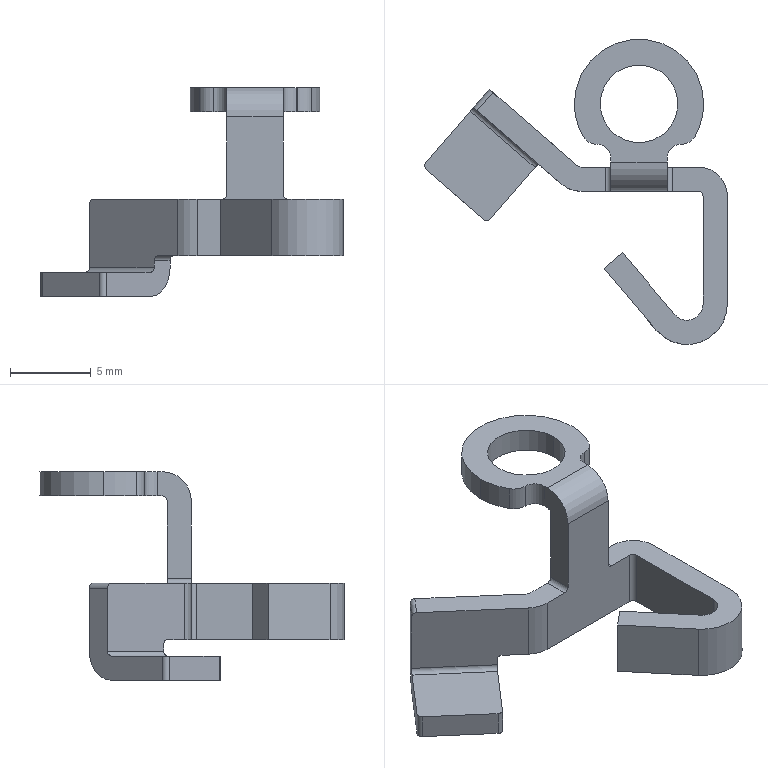Part | STEP file | TQ-DD-1105-THTerminalC1010_デフォルト | 1 solid | 48 faces | box 18.722 x 18.871 x 12.9 mm | volume 306.798 mm3 | cylinder 25 | plane 23 | commonest cylinder face diameters 0.6 x10 3.6 x4 2 x3 8 x3 1.6 x2 4.8 x2
STEP:
#1=CARTESIAN_POINT('',(-2.4,0.,0.));
#2=VERTEX_POINT('',#1);
#3=CARTESIAN_POINT('',(2.4,0.,0.));
#4=VERTEX_POINT('',#3);
#5=CARTESIAN_POINT('',(0.,0.,0.));
#6=DIRECTION('',(0.,0.,1.));
#7=DIRECTION('',(1.,0.,0.));
#8=AXIS2_PLACEMENT_3D('',#5,#6,#7);
#9=CIRCLE('',#8,2.4);
#10=EDGE_CURVE('',#2,#4,#9,.T.);
#11=ORIENTED_EDGE('',*,*,#10,.F.);
#12=CARTESIAN_POINT('',(-2.4,0.,1.5));
#13=VERTEX_POINT('',#12);
#14=CARTESIAN_POINT('',(-2.4,0.,0.75));
#15=DIRECTION('',(0.,0.,1.));
#16=VECTOR('',#15,1000.);
#17=LINE('',#14,#16);
#18=EDGE_CURVE('',#2,#13,#17,.T.);
#19=ORIENTED_EDGE('',*,*,#18,.T.);
#20=CARTESIAN_POINT('',(2.4,0.,1.5));
#21=VERTEX_POINT('',#20);
#22=CARTESIAN_POINT('',(0.,0.,1.5));
#23=DIRECTION('',(0.,0.,-1.));
#24=DIRECTION('',(1.,0.,0.));
#25=AXIS2_PLACEMENT_3D('',#22,#23,#24);
#26=CIRCLE('',#25,2.4);
#27=EDGE_CURVE('',#21,#13,#26,.T.);
#28=ORIENTED_EDGE('',*,*,#27,.F.);
#29=CARTESIAN_POINT('',(2.4,0.,0.75));
#30=DIRECTION('',(0.,0.,1.));
#31=VECTOR('',#30,1000.);
#32=LINE('',#29,#31);
#33=EDGE_CURVE('',#4,#21,#32,.T.);
#34=ORIENTED_EDGE('',*,*,#33,.F.);
#35=EDGE_LOOP('',(#11,#19,#28,#34));
#36=FACE_OUTER_BOUND('',#35,.T.);
#37=CARTESIAN_POINT('',(0.,0.,0.75));
#38=DIRECTION('',(0.,0.,1.));
#39=DIRECTION('',(1.,0.,0.));
#40=AXIS2_PLACEMENT_3D('',#37,#38,#39);
#41=CYLINDRICAL_SURFACE('',#40,2.4);
#42=ADVANCED_FACE('',(#36),#41,.F.);
#43=CARTESIAN_POINT('',(4.,0.,0.));
#44=VERTEX_POINT('',#43);
#45=CARTESIAN_POINT('',(-4.,0.,0.));
#46=VERTEX_POINT('',#45);
#47=CARTESIAN_POINT('',(0.,0.,0.));
#48=DIRECTION('',(0.,0.,1.));
#49=DIRECTION('',(1.,0.,0.));
#50=AXIS2_PLACEMENT_3D('',#47,#48,#49);
#51=CIRCLE('',#50,4.);
#52=EDGE_CURVE('',#44,#46,#51,.T.);
#53=ORIENTED_EDGE('',*,*,#52,.T.);
#54=CARTESIAN_POINT('',(-4.,0.,1.5));
#55=VERTEX_POINT('',#54);
#56=CARTESIAN_POINT('',(-4.,0.,0.75));
#57=DIRECTION('',(0.,0.,1.));
#58=VECTOR('',#57,1000.);
#59=LINE('',#56,#58);
#60=EDGE_CURVE('',#46,#55,#59,.T.);
#61=ORIENTED_EDGE('',*,*,#60,.T.);
#62=CARTESIAN_POINT('',(4.,0.,1.5));
#63=VERTEX_POINT('',#62);
#64=CARTESIAN_POINT('',(0.,0.,1.5));
#65=DIRECTION('',(0.,0.,1.));
#66=DIRECTION('',(1.,0.,0.));
#67=AXIS2_PLACEMENT_3D('',#64,#65,#66);
#68=CIRCLE('',#67,4.);
#69=EDGE_CURVE('',#63,#55,#68,.T.);
#70=ORIENTED_EDGE('',*,*,#69,.F.);
#71=CARTESIAN_POINT('',(4.,0.,0.75));
#72=DIRECTION('',(0.,0.,1.));
#73=VECTOR('',#72,1000.);
#74=LINE('',#71,#73);
#75=EDGE_CURVE('',#44,#63,#74,.T.);
#76=ORIENTED_EDGE('',*,*,#75,.F.);
#77=EDGE_LOOP('',(#53,#61,#70,#76));
#78=FACE_OUTER_BOUND('',#77,.T.);
#79=CARTESIAN_POINT('',(0.,0.,0.75));
#80=DIRECTION('',(0.,0.,1.));
#81=DIRECTION('',(1.,0.,0.));
#82=AXIS2_PLACEMENT_3D('',#79,#80,#81);
#83=CYLINDRICAL_SURFACE('',#82,4.);
#84=ADVANCED_FACE('',(#78),#83,.T.);
#85=CARTESIAN_POINT('',(3.464,-2.,0.));
#86=VERTEX_POINT('',#85);
#87=CARTESIAN_POINT('',(0.,0.,0.));
#88=DIRECTION('',(0.,0.,1.));
#89=DIRECTION('',(1.,0.,0.));
#90=AXIS2_PLACEMENT_3D('',#87,#88,#89);
#91=CIRCLE('',#90,4.);
#92=EDGE_CURVE('',#86,#44,#91,.T.);
#93=ORIENTED_EDGE('',*,*,#92,.T.);
#94=ORIENTED_EDGE('',*,*,#75,.T.);
#95=CARTESIAN_POINT('',(3.464,-2.,1.5));
#96=VERTEX_POINT('',#95);
#97=CARTESIAN_POINT('',(0.,0.,1.5));
#98=DIRECTION('',(0.,0.,1.));
#99=DIRECTION('',(1.,0.,0.));
#100=AXIS2_PLACEMENT_3D('',#97,#98,#99);
#101=CIRCLE('',#100,4.);
#102=EDGE_CURVE('',#96,#63,#101,.T.);
#103=ORIENTED_EDGE('',*,*,#102,.F.);
#104=CARTESIAN_POINT('',(3.464,-2.,0.75));
#105=DIRECTION('',(0.,0.,1.));
#106=VECTOR('',#105,1000.);
#107=LINE('',#104,#106);
#108=EDGE_CURVE('',#86,#96,#107,.T.);
#109=ORIENTED_EDGE('',*,*,#108,.F.);
#110=EDGE_LOOP('',(#93,#94,#103,#109));
#111=FACE_OUTER_BOUND('',#110,.T.);
#112=CARTESIAN_POINT('',(0.,0.,0.75));
#113=DIRECTION('',(0.,0.,1.));
#114=DIRECTION('',(1.,0.,0.));
#115=AXIS2_PLACEMENT_3D('',#112,#113,#114);
#116=CYLINDRICAL_SURFACE('',#115,4.);
#117=ADVANCED_FACE('',(#111),#116,.T.);
#118=CARTESIAN_POINT('',(1.75,-5.4,-0.3));
#119=VERTEX_POINT('',#118);
#120=CARTESIAN_POINT('',(-1.75,-5.4,-0.3));
#121=VERTEX_POINT('',#120);
#122=CARTESIAN_POINT('',(-1.75,-5.4,-0.3));
#123=DIRECTION('',(-1.,0.,0.));
#124=VECTOR('',#123,1000.);
#125=LINE('',#122,#124);
#126=EDGE_CURVE('',#119,#121,#125,.T.);
#127=ORIENTED_EDGE('',*,*,#126,.T.);
#128=CARTESIAN_POINT('',(-1.75,-5.4,-5.1));
#129=VERTEX_POINT('',#128);
#130=CARTESIAN_POINT('',(-1.75,-5.4,0.));
#131=DIRECTION('',(0.,0.,-1.));
#132=VECTOR('',#131,1000.);
#133=LINE('',#130,#132);
#134=EDGE_CURVE('',#121,#129,#133,.T.);
#135=ORIENTED_EDGE('',*,*,#134,.T.);
#136=CARTESIAN_POINT('',(-2.05,-5.4,-5.4));
#137=VERTEX_POINT('',#136);
#138=CARTESIAN_POINT('',(-2.05,-5.4,-5.1));
#139=DIRECTION('',(0.,1.,0.));
#140=DIRECTION('',(0.,0.,-1.));
#141=AXIS2_PLACEMENT_3D('',#138,#139,#140);
#142=CIRCLE('',#141,0.3);
#143=EDGE_CURVE('',#129,#137,#142,.T.);
#144=ORIENTED_EDGE('',*,*,#143,.T.);
#145=CARTESIAN_POINT('',(-3.588,-5.4,-5.4));
#146=VERTEX_POINT('',#145);
#147=CARTESIAN_POINT('',(0.,-5.4,-5.4));
#148=DIRECTION('',(-1.,0.,0.));
#149=VECTOR('',#148,1000.);
#150=LINE('',#147,#149);
#151=EDGE_CURVE('',#137,#146,#150,.T.);
#152=ORIENTED_EDGE('',*,*,#151,.T.);
#153=CARTESIAN_POINT('',(-3.588,-5.4,-8.9));
#154=VERTEX_POINT('',#153);
#155=CARTESIAN_POINT('',(-3.588,-5.4,0.));
#156=DIRECTION('',(0.,0.,-1.));
#157=VECTOR('',#156,1000.);
#158=LINE('',#155,#157);
#159=EDGE_CURVE('',#146,#154,#158,.T.);
#160=ORIENTED_EDGE('',*,*,#159,.T.);
#161=CARTESIAN_POINT('',(3.663,-5.4,-8.9));
#162=VERTEX_POINT('',#161);
#163=CARTESIAN_POINT('',(-1.75,-5.4,-8.9));
#164=DIRECTION('',(1.,0.,0.));
#165=VECTOR('',#164,1000.);
#166=LINE('',#163,#165);
#167=EDGE_CURVE('',#154,#162,#166,.T.);
#168=ORIENTED_EDGE('',*,*,#167,.T.);
#169=CARTESIAN_POINT('',(3.663,-5.4,-5.4));
#170=VERTEX_POINT('',#169);
#171=CARTESIAN_POINT('',(3.663,-5.4,0.));
#172=DIRECTION('',(0.,0.,1.));
#173=VECTOR('',#172,1000.);
#174=LINE('',#171,#173);
#175=EDGE_CURVE('',#162,#170,#174,.T.);
#176=ORIENTED_EDGE('',*,*,#175,.T.);
#177=CARTESIAN_POINT('',(2.05,-5.4,-5.4));
#178=VERTEX_POINT('',#177);
#179=CARTESIAN_POINT('',(0.,-5.4,-5.4));
#180=DIRECTION('',(-1.,0.,0.));
#181=VECTOR('',#180,1000.);
#182=LINE('',#179,#181);
#183=EDGE_CURVE('',#170,#178,#182,.T.);
#184=ORIENTED_EDGE('',*,*,#183,.T.);
#185=CARTESIAN_POINT('',(1.75,-5.4,-5.1));
#186=VERTEX_POINT('',#185);
#187=CARTESIAN_POINT('',(2.05,-5.4,-5.1));
#188=DIRECTION('',(0.,1.,0.));
#189=DIRECTION('',(0.,0.,1.));
#190=AXIS2_PLACEMENT_3D('',#187,#188,#189);
#191=CIRCLE('',#190,0.3);
#192=EDGE_CURVE('',#178,#186,#191,.T.);
#193=ORIENTED_EDGE('',*,*,#192,.T.);
#194=CARTESIAN_POINT('',(1.75,-5.4,0.));
#195=DIRECTION('',(0.,0.,1.));
#196=VECTOR('',#195,1000.);
#197=LINE('',#194,#196);
#198=EDGE_CURVE('',#186,#119,#197,.T.);
#199=ORIENTED_EDGE('',*,*,#198,.T.);
#200=EDGE_LOOP('',(#127,#135,#144,#152,#160,#168,#176,#184,#193,#199));
#201=FACE_OUTER_BOUND('',#200,.T.);
#202=CARTESIAN_POINT('',(-1.75,-5.4,0.));
#203=DIRECTION('',(0.,-1.,0.));
#204=DIRECTION('',(0.,0.,-1.));
#205=AXIS2_PLACEMENT_3D('',#202,#203,#204);
#206=PLANE('',#205);
#207=ADVANCED_FACE('',(#201),#206,.T.);
#208=CARTESIAN_POINT('',(-1.75,-3.9,-0.3));
#209=VERTEX_POINT('',#208);
#210=CARTESIAN_POINT('',(-1.75,-3.9,-5.1));
#211=VERTEX_POINT('',#210);
#212=CARTESIAN_POINT('',(-1.75,-3.9,0.));
#213=DIRECTION('',(0.,0.,-1.));
#214=VECTOR('',#213,1000.);
#215=LINE('',#212,#214);
#216=EDGE_CURVE('',#209,#211,#215,.T.);
#217=ORIENTED_EDGE('',*,*,#216,.T.);
#218=CARTESIAN_POINT('',(-1.75,-2.5,-5.1));
#219=DIRECTION('',(0.,-1.,0.));
#220=VECTOR('',#219,1000.);
#221=LINE('',#218,#220);
#222=EDGE_CURVE('',#211,#129,#221,.T.);
#223=ORIENTED_EDGE('',*,*,#222,.T.);
#224=ORIENTED_EDGE('',*,*,#134,.F.);
#225=CARTESIAN_POINT('',(-1.75,-3.6,1.5));
#226=VERTEX_POINT('',#225);
#227=CARTESIAN_POINT('',(-1.75,-3.6,-0.3));
#228=DIRECTION('',(-1.,0.,0.));
#229=DIRECTION('',(0.,0.,-1.));
#230=AXIS2_PLACEMENT_3D('',#227,#228,#229);
#231=CIRCLE('',#230,1.8);
#232=EDGE_CURVE('',#121,#226,#231,.T.);
#233=ORIENTED_EDGE('',*,*,#232,.T.);
#234=CARTESIAN_POINT('',(-1.75,-3.3,1.5));
#235=VERTEX_POINT('',#234);
#236=CARTESIAN_POINT('',(-1.75,0.,1.5));
#237=DIRECTION('',(0.,-1.,0.));
#238=VECTOR('',#237,1000.);
#239=LINE('',#236,#238);
#240=EDGE_CURVE('',#235,#226,#239,.T.);
#241=ORIENTED_EDGE('',*,*,#240,.F.);
#242=CARTESIAN_POINT('',(-1.75,-3.3,0.));
#243=VERTEX_POINT('',#242);
#244=CARTESIAN_POINT('',(-1.75,-3.3,0.));
#245=DIRECTION('',(0.,0.,-1.));
#246=VECTOR('',#245,1000.);
#247=LINE('',#244,#246);
#248=EDGE_CURVE('',#235,#243,#247,.T.);
#249=ORIENTED_EDGE('',*,*,#248,.T.);
#250=CARTESIAN_POINT('',(-1.75,-3.6,0.));
#251=VERTEX_POINT('',#250);
#252=CARTESIAN_POINT('',(-1.75,0.,0.));
#253=DIRECTION('',(0.,-1.,0.));
#254=VECTOR('',#253,1000.);
#255=LINE('',#252,#254);
#256=EDGE_CURVE('',#243,#251,#255,.T.);
#257=ORIENTED_EDGE('',*,*,#256,.T.);
#258=CARTESIAN_POINT('',(-1.75,-3.6,-0.3));
#259=DIRECTION('',(1.,0.,0.));
#260=DIRECTION('',(0.,0.,1.));
#261=AXIS2_PLACEMENT_3D('',#258,#259,#260);
#262=CIRCLE('',#261,0.3);
#263=EDGE_CURVE('',#251,#209,#262,.T.);
#264=ORIENTED_EDGE('',*,*,#263,.T.);
#265=EDGE_LOOP('',(#217,#223,#224,#233,#241,#249,#257,#264));
#266=FACE_OUTER_BOUND('',#265,.T.);
#267=CARTESIAN_POINT('',(-1.75,-2.5,0.));
#268=DIRECTION('',(-1.,0.,0.));
#269=DIRECTION('',(0.,0.,1.));
#270=AXIS2_PLACEMENT_3D('',#267,#268,#269);
#271=PLANE('',#270);
#272=ADVANCED_FACE('',(#266),#271,.T.);
#273=ORIENTED_EDGE('',*,*,#232,.F.);
#274=ORIENTED_EDGE('',*,*,#126,.F.);
#275=CARTESIAN_POINT('',(1.75,-3.6,1.5));
#276=VERTEX_POINT('',#275);
#277=CARTESIAN_POINT('',(1.75,-3.6,-0.3));
#278=DIRECTION('',(-1.,0.,0.));
#279=DIRECTION('',(0.,0.,-1.));
#280=AXIS2_PLACEMENT_3D('',#277,#278,#279);
#281=CIRCLE('',#280,1.8);
#282=EDGE_CURVE('',#119,#276,#281,.T.);
#283=ORIENTED_EDGE('',*,*,#282,.T.);
#284=CARTESIAN_POINT('',(0.,-3.6,1.5));
#285=DIRECTION('',(-1.,0.,0.));
#286=VECTOR('',#285,1000.);
#287=LINE('',#284,#286);
#288=EDGE_CURVE('',#276,#226,#287,.T.);
#289=ORIENTED_EDGE('',*,*,#288,.T.);
#290=EDGE_LOOP('',(#273,#274,#283,#289));
#291=FACE_OUTER_BOUND('',#290,.T.);
#292=CARTESIAN_POINT('',(0.,-3.6,-0.3));
#293=DIRECTION('',(1.,0.,0.));
#294=DIRECTION('',(0.,0.,-1.));
#295=AXIS2_PLACEMENT_3D('',#292,#293,#294);
#296=CYLINDRICAL_SURFACE('',#295,1.8);
#297=ADVANCED_FACE('',(#291),#296,.T.);
#298=ORIENTED_EDGE('',*,*,#198,.F.);
#299=CARTESIAN_POINT('',(1.75,-3.9,-5.1));
#300=VERTEX_POINT('',#299);
#301=CARTESIAN_POINT('',(1.75,-5.4,-5.1));
#302=DIRECTION('',(0.,1.,0.));
#303=VECTOR('',#302,1000.);
#304=LINE('',#301,#303);
#305=EDGE_CURVE('',#186,#300,#304,.T.);
#306=ORIENTED_EDGE('',*,*,#305,.T.);
#307=CARTESIAN_POINT('',(1.75,-3.9,-0.3));
#308=VERTEX_POINT('',#307);
#309=CARTESIAN_POINT('',(1.75,-3.9,0.));
#310=DIRECTION('',(0.,0.,1.));
#311=VECTOR('',#310,1000.);
#312=LINE('',#309,#311);
#313=EDGE_CURVE('',#300,#308,#312,.T.);
#314=ORIENTED_EDGE('',*,*,#313,.T.);
#315=CARTESIAN_POINT('',(1.75,-3.6,0.));
#316=VERTEX_POINT('',#315);
#317=CARTESIAN_POINT('',(1.75,-3.6,-0.3));
#318=DIRECTION('',(-1.,0.,0.));
#319=DIRECTION('',(0.,0.,1.));
#320=AXIS2_PLACEMENT_3D('',#317,#318,#319);
#321=CIRCLE('',#320,0.3);
#322=EDGE_CURVE('',#308,#316,#321,.T.);
#323=ORIENTED_EDGE('',*,*,#322,.T.);
#324=CARTESIAN_POINT('',(1.75,-3.3,0.));
#325=VERTEX_POINT('',#324);
#326=CARTESIAN_POINT('',(1.75,0.,0.));
#327=DIRECTION('',(0.,1.,0.));
#328=VECTOR('',#327,1000.);
#329=LINE('',#326,#328);
#330=EDGE_CURVE('',#316,#325,#329,.T.);
#331=ORIENTED_EDGE('',*,*,#330,.T.);
#332=CARTESIAN_POINT('',(1.75,-3.3,1.5));
#333=VERTEX_POINT('',#332);
#334=CARTESIAN_POINT('',(1.75,-3.3,0.));
#335=DIRECTION('',(0.,0.,1.));
#336=VECTOR('',#335,1000.);
#337=LINE('',#334,#336);
#338=EDGE_CURVE('',#325,#333,#337,.T.);
#339=ORIENTED_EDGE('',*,*,#338,.T.);
#340=CARTESIAN_POINT('',(1.75,-5.4,1.5));
#341=DIRECTION('',(0.,-1.,0.));
#342=VECTOR('',#341,1000.);
#343=LINE('',#340,#342);
#344=EDGE_CURVE('',#333,#276,#343,.T.);
#345=ORIENTED_EDGE('',*,*,#344,.T.);
#346=ORIENTED_EDGE('',*,*,#282,.F.);
#347=EDGE_LOOP('',(#298,#306,#314,#323,#331,#339,#345,#346));
#348=FACE_OUTER_BOUND('',#347,.T.);
#349=CARTESIAN_POINT('',(1.75,-5.4,0.));
#350=DIRECTION('',(1.,0.,0.));
#351=DIRECTION('',(0.,0.,-1.));
#352=AXIS2_PLACEMENT_3D('',#349,#350,#351);
#353=PLANE('',#352);
#354=ADVANCED_FACE('',(#348),#353,.T.);
#355=ORIENTED_EDGE('',*,*,#175,.F.);
#356=CARTESIAN_POINT('',(3.963,-5.7,-8.9));
#357=VERTEX_POINT('',#356);
#358=CARTESIAN_POINT('',(3.663,-5.7,-8.9));
#359=DIRECTION('',(0.,0.,1.));
#360=DIRECTION('',(-1.,0.,0.));
#361=AXIS2_PLACEMENT_3D('',#358,#359,#360);
#362=CIRCLE('',#361,0.3);
#363=EDGE_CURVE('',#357,#162,#362,.T.);
#364=ORIENTED_EDGE('',*,*,#363,.F.);
#365=CARTESIAN_POINT('',(3.963,-5.7,-5.4));
#366=VERTEX_POINT('',#365);
#367=CARTESIAN_POINT('',(3.963,-5.7,-7.15));
#368=DIRECTION('',(0.,0.,-1.));
#369=VECTOR('',#368,1000.);
#370=LINE('',#367,#369);
#371=EDGE_CURVE('',#366,#357,#370,.T.);
#372=ORIENTED_EDGE('',*,*,#371,.F.);
#373=CARTESIAN_POINT('',(3.663,-5.7,-5.4));
#374=DIRECTION('',(0.,0.,1.));
#375=DIRECTION('',(-1.,0.,0.));
#376=AXIS2_PLACEMENT_3D('',#373,#374,#375);
#377=CIRCLE('',#376,0.3);
#378=EDGE_CURVE('',#366,#170,#377,.T.);
#379=ORIENTED_EDGE('',*,*,#378,.T.);
#380=EDGE_LOOP('',(#355,#364,#372,#379));
#381=FACE_OUTER_BOUND('',#380,.T.);
#382=CARTESIAN_POINT('',(3.663,-5.7,-7.15));
#383=DIRECTION('',(0.,0.,-1.));
#384=DIRECTION('',(-1.,0.,0.));
#385=AXIS2_PLACEMENT_3D('',#382,#383,#384);
#386=CYLINDRICAL_SURFACE('',#385,0.3);
#387=ADVANCED_FACE('',(#381),#386,.F.);
#388=CARTESIAN_POINT('',(-4.766,-4.962,-8.9));
#389=VERTEX_POINT('',#388);
#390=CARTESIAN_POINT('',(-6.006,-3.889,-8.9));
#391=VERTEX_POINT('',#390);
#392=CARTESIAN_POINT('',(-4.766,-4.962,-8.9));
#393=DIRECTION('',(-0.7564,0.6541,0.));
#394=VECTOR('',#393,1000.);
#395=LINE('',#392,#394);
#396=EDGE_CURVE('',#389,#391,#395,.T.);
#397=ORIENTED_EDGE('',*,*,#396,.T.);
#398=CARTESIAN_POINT('',(-5.025,-2.754,-8.9));
#399=VERTEX_POINT('',#398);
#400=CARTESIAN_POINT('',(-6.006,-3.889,-8.9));
#401=DIRECTION('',(0.6541,0.7564,0.));
#402=VECTOR('',#401,1000.);
#403=LINE('',#400,#402);
#404=EDGE_CURVE('',#391,#399,#403,.T.);
#405=ORIENTED_EDGE('',*,*,#404,.T.);
#406=CARTESIAN_POINT('',(-3.785,-3.827,-8.9));
#407=VERTEX_POINT('',#406);
#408=CARTESIAN_POINT('',(-9.261,0.9089,-8.9));
#409=DIRECTION('',(0.7564,-0.6541,0.));
#410=VECTOR('',#409,1000.);
#411=LINE('',#408,#410);
#412=EDGE_CURVE('',#399,#407,#411,.T.);
#413=ORIENTED_EDGE('',*,*,#412,.T.);
#414=CARTESIAN_POINT('',(-3.588,-3.9,-8.9));
#415=VERTEX_POINT('',#414);
#416=CARTESIAN_POINT('',(-3.588,-3.6,-8.9));
#417=DIRECTION('',(0.,0.,1.));
#418=DIRECTION('',(-1.,0.,0.));
#419=AXIS2_PLACEMENT_3D('',#416,#417,#418);
#420=CIRCLE('',#419,0.3);
#421=EDGE_CURVE('',#407,#415,#420,.T.);
#422=ORIENTED_EDGE('',*,*,#421,.T.);
#423=CARTESIAN_POINT('',(3.663,-3.9,-8.9));
#424=VERTEX_POINT('',#423);
#425=CARTESIAN_POINT('',(0.,-3.9,-8.9));
#426=DIRECTION('',(1.,0.,0.));
#427=VECTOR('',#426,1000.);
#428=LINE('',#425,#427);
#429=EDGE_CURVE('',#415,#424,#428,.T.);
#430=ORIENTED_EDGE('',*,*,#429,.T.);
#431=CARTESIAN_POINT('',(5.463,-5.7,-8.9));
#432=VERTEX_POINT('',#431);
#433=CARTESIAN_POINT('',(3.663,-5.7,-8.9));
#434=DIRECTION('',(0.,0.,-1.));
#435=DIRECTION('',(-1.,0.,0.));
#436=AXIS2_PLACEMENT_3D('',#433,#434,#435);
#437=CIRCLE('',#436,1.8);
#438=EDGE_CURVE('',#424,#432,#437,.T.);
#439=ORIENTED_EDGE('',*,*,#438,.T.);
#440=CARTESIAN_POINT('',(5.463,-12.371,-8.9));
#441=VERTEX_POINT('',#440);
#442=CARTESIAN_POINT('',(5.463,-5.4,-8.9));
#443=DIRECTION('',(0.,-1.,0.));
#444=VECTOR('',#443,1000.);
#445=LINE('',#442,#444);
#446=EDGE_CURVE('',#432,#441,#445,.T.);
#447=ORIENTED_EDGE('',*,*,#446,.T.);
#448=CARTESIAN_POINT('',(1.048,-13.978,-8.9));
#449=VERTEX_POINT('',#448);
#450=CARTESIAN_POINT('',(2.963,-12.371,-8.9));
#451=DIRECTION('',(0.,0.,-1.));
#452=DIRECTION('',(-1.,0.,0.));
#453=AXIS2_PLACEMENT_3D('',#450,#451,#452);
#454=CIRCLE('',#453,2.5);
#455=EDGE_CURVE('',#441,#449,#454,.T.);
#456=ORIENTED_EDGE('',*,*,#455,.T.);
#457=CARTESIAN_POINT('',(-2.166,-10.147,-8.9));
#458=VERTEX_POINT('',#457);
#459=CARTESIAN_POINT('',(1.048,-13.978,-8.9));
#460=DIRECTION('',(-0.6428,0.766,0.));
#461=VECTOR('',#460,1000.);
#462=LINE('',#459,#461);
#463=EDGE_CURVE('',#449,#458,#462,.T.);
#464=ORIENTED_EDGE('',*,*,#463,.T.);
#465=CARTESIAN_POINT('',(-1.017,-9.183,-8.9));
#466=VERTEX_POINT('',#465);
#467=CARTESIAN_POINT('',(-1.017,-9.183,-8.9));
#468=DIRECTION('',(-0.766,-0.6428,0.));
#469=VECTOR('',#468,1000.);
#470=LINE('',#467,#469);
#471=EDGE_CURVE('',#466,#458,#470,.T.);
#472=ORIENTED_EDGE('',*,*,#471,.F.);
#473=CARTESIAN_POINT('',(2.197,-13.013,-8.9));
#474=VERTEX_POINT('',#473);
#475=CARTESIAN_POINT('',(-1.017,-9.183,-8.9));
#476=DIRECTION('',(0.6428,-0.766,0.));
#477=VECTOR('',#476,1000.);
#478=LINE('',#475,#477);
#479=EDGE_CURVE('',#466,#474,#478,.T.);
#480=ORIENTED_EDGE('',*,*,#479,.T.);
#481=CARTESIAN_POINT('',(3.963,-12.371,-8.9));
#482=VERTEX_POINT('',#481);
#483=CARTESIAN_POINT('',(2.963,-12.371,-8.9));
#484=DIRECTION('',(0.,0.,1.));
#485=DIRECTION('',(-1.,0.,0.));
#486=AXIS2_PLACEMENT_3D('',#483,#484,#485);
#487=CIRCLE('',#486,1.);
#488=EDGE_CURVE('',#474,#482,#487,.T.);
#489=ORIENTED_EDGE('',*,*,#488,.T.);
#490=CARTESIAN_POINT('',(3.963,-5.4,-8.9));
#491=DIRECTION('',(0.,1.,0.));
#492=VECTOR('',#491,1000.);
#493=LINE('',#490,#492);
#494=EDGE_CURVE('',#482,#357,#493,.T.);
#495=ORIENTED_EDGE('',*,*,#494,.T.);
#496=ORIENTED_EDGE('',*,*,#363,.T.);
#497=ORIENTED_EDGE('',*,*,#167,.F.);
#498=CARTESIAN_POINT('',(-3.588,-3.6,-8.9));
#499=DIRECTION('',(0.,0.,-1.));
#500=DIRECTION('',(-1.,0.,0.));
#501=AXIS2_PLACEMENT_3D('',#498,#499,#500);
#502=CIRCLE('',#501,1.8);
#503=EDGE_CURVE('',#154,#389,#502,.T.);
#504=ORIENTED_EDGE('',*,*,#503,.T.);
#505=EDGE_LOOP('',(#397,#405,#413,#422,#430,#439,#447,#456,#464,#472,#480,#489,#495,#496,#497,#504));
#506=FACE_OUTER_BOUND('',#505,.T.);
#507=CARTESIAN_POINT('',(0.,-5.4,-8.9));
#508=DIRECTION('',(0.,0.,-1.));
#509=DIRECTION('',(-1.,0.,0.));
#510=AXIS2_PLACEMENT_3D('',#507,#508,#509);
#511=PLANE('',#510);
#512=ADVANCED_FACE('',(#506),#511,.T.);
#513=ORIENTED_EDGE('',*,*,#503,.F.);
#514=ORIENTED_EDGE('',*,*,#159,.F.);
#515=CARTESIAN_POINT('',(-4.766,-4.962,-5.4));
#516=VERTEX_POINT('',#515);
#517=CARTESIAN_POINT('',(-3.588,-3.6,-5.4));
#518=DIRECTION('',(0.,0.,-1.));
#519=DIRECTION('',(-1.,0.,0.));
#520=AXIS2_PLACEMENT_3D('',#517,#518,#519);
#521=CIRCLE('',#520,1.8);
#522=EDGE_CURVE('',#146,#516,#521,.T.);
#523=ORIENTED_EDGE('',*,*,#522,.T.);
#524=CARTESIAN_POINT('',(-4.766,-4.962,-7.15));
#525=DIRECTION('',(0.,0.,-1.));
#526=VECTOR('',#525,1000.);
#527=LINE('',#524,#526);
#528=EDGE_CURVE('',#516,#389,#527,.T.);
#529=ORIENTED_EDGE('',*,*,#528,.T.);
#530=EDGE_LOOP('',(#513,#514,#523,#529));
#531=FACE_OUTER_BOUND('',#530,.T.);
#532=CARTESIAN_POINT('',(-3.588,-3.6,-7.15));
#533=DIRECTION('',(0.,0.,-1.));
#534=DIRECTION('',(-1.,0.,0.));
#535=AXIS2_PLACEMENT_3D('',#532,#533,#534);
#536=CYLINDRICAL_SURFACE('',#535,1.8);
#537=ADVANCED_FACE('',(#531),#536,.T.);
#538=ORIENTED_EDGE('',*,*,#143,.F.);
#539=ORIENTED_EDGE('',*,*,#222,.F.);
#540=CARTESIAN_POINT('',(-2.05,-3.9,-5.4));
#541=VERTEX_POINT('',#540);
#542=CARTESIAN_POINT('',(-2.05,-3.9,-5.1));
#543=DIRECTION('',(0.,-1.,0.));
#544=DIRECTION('',(0.,0.,-1.));
#545=AXIS2_PLACEMENT_3D('',#542,#543,#544);
#546=CIRCLE('',#545,0.3);
#547=EDGE_CURVE('',#541,#211,#546,.T.);
#548=ORIENTED_EDGE('',*,*,#547,.F.);
#549=CARTESIAN_POINT('',(-2.05,0.,-5.4));
#550=DIRECTION('',(0.,-1.,0.));
#551=VECTOR('',#550,1000.);
#552=LINE('',#549,#551);
#553=EDGE_CURVE('',#541,#137,#552,.T.);
#554=ORIENTED_EDGE('',*,*,#553,.T.);
#555=EDGE_LOOP('',(#538,#539,#548,#554));
#556=FACE_OUTER_BOUND('',#555,.T.);
#557=CARTESIAN_POINT('',(-2.05,-2.246,-5.1));
#558=DIRECTION('',(0.,-1.,0.));
#559=DIRECTION('',(0.,0.,-1.));
#560=AXIS2_PLACEMENT_3D('',#557,#558,#559);
#561=CYLINDRICAL_SURFACE('',#560,0.3);
#562=ADVANCED_FACE('',(#556),#561,.F.);
#563=CARTESIAN_POINT('',(0.,-3.9,-0.3));
#564=DIRECTION('',(-1.,0.,0.));
#565=VECTOR('',#564,1000.);
#566=LINE('',#563,#565);
#567=EDGE_CURVE('',#308,#209,#566,.T.);
#568=ORIENTED_EDGE('',*,*,#567,.F.);
#569=ORIENTED_EDGE('',*,*,#313,.F.);
#570=CARTESIAN_POINT('',(2.05,-3.9,-5.4));
#571=VERTEX_POINT('',#570);
#572=CARTESIAN_POINT('',(2.05,-3.9,-5.1));
#573=DIRECTION('',(0.,1.,0.));
#574=DIRECTION('',(0.,0.,1.));
#575=AXIS2_PLACEMENT_3D('',#572,#573,#574);
#576=CIRCLE('',#575,0.3);
#577=EDGE_CURVE('',#571,#300,#576,.T.);
#578=ORIENTED_EDGE('',*,*,#577,.F.);
#579=CARTESIAN_POINT('',(3.663,-3.9,-5.4));
#580=VERTEX_POINT('',#579);
#581=CARTESIAN_POINT('',(0.,-3.9,-5.4));
#582=DIRECTION('',(1.,0.,0.));
#583=VECTOR('',#582,1000.);
#584=LINE('',#581,#583);
#585=EDGE_CURVE('',#571,#580,#584,.T.);
#586=ORIENTED_EDGE('',*,*,#585,.T.);
#587=CARTESIAN_POINT('',(3.663,-3.9,1.5));
#588=DIRECTION('',(0.,0.,1.));
#589=VECTOR('',#588,1000.);
#590=LINE('',#587,#589);
#591=EDGE_CURVE('',#424,#580,#590,.T.);
#592=ORIENTED_EDGE('',*,*,#591,.F.);
#593=ORIENTED_EDGE('',*,*,#429,.F.);
#594=CARTESIAN_POINT('',(-3.588,-3.9,-5.4));
#595=VERTEX_POINT('',#594);
#596=CARTESIAN_POINT('',(-3.588,-3.9,1.5));
#597=DIRECTION('',(0.,0.,-1.));
#598=VECTOR('',#597,1000.);
#599=LINE('',#596,#598);
#600=EDGE_CURVE('',#595,#415,#599,.T.);
#601=ORIENTED_EDGE('',*,*,#600,.F.);
#602=CARTESIAN_POINT('',(0.,-3.9,-5.4));
#603=DIRECTION('',(1.,0.,0.));
#604=VECTOR('',#603,1000.);
#605=LINE('',#602,#604);
#606=EDGE_CURVE('',#595,#541,#605,.T.);
#607=ORIENTED_EDGE('',*,*,#606,.T.);
#608=ORIENTED_EDGE('',*,*,#547,.T.);
#609=ORIENTED_EDGE('',*,*,#216,.F.);
#610=EDGE_LOOP('',(#568,#569,#578,#586,#592,#593,#601,#607,#608,#609));
#611=FACE_OUTER_BOUND('',#610,.T.);
#612=CARTESIAN_POINT('',(0.,-3.9,1.5));
#613=DIRECTION('',(0.,-1.,0.));
#614=DIRECTION('',(0.,0.,-1.));
#615=AXIS2_PLACEMENT_3D('',#612,#613,#614);
#616=PLANE('',#615);
#617=ADVANCED_FACE('',(#611),#616,.F.);
#618=CARTESIAN_POINT('',(-2.55,-2.5,1.5));
#619=VERTEX_POINT('',#618);
#620=CARTESIAN_POINT('',(-2.55,-3.3,1.5));
#621=DIRECTION('',(0.,0.,-1.));
#622=DIRECTION('',(1.,0.,0.));
#623=AXIS2_PLACEMENT_3D('',#620,#621,#622);
#624=CIRCLE('',#623,0.8);
#625=EDGE_CURVE('',#619,#235,#624,.T.);
#626=ORIENTED_EDGE('',*,*,#625,.F.);
#627=CARTESIAN_POINT('',(-2.55,-2.5,0.));
#628=VERTEX_POINT('',#627);
#629=CARTESIAN_POINT('',(-2.55,-2.5,-3.7));
#630=DIRECTION('',(0.,0.,1.));
#631=VECTOR('',#630,1000.);
#632=LINE('',#629,#631);
#633=EDGE_CURVE('',#628,#619,#632,.T.);
#634=ORIENTED_EDGE('',*,*,#633,.F.);
#635=CARTESIAN_POINT('',(-2.55,-3.3,0.));
#636=DIRECTION('',(0.,0.,-1.));
#637=DIRECTION('',(1.,0.,0.));
#638=AXIS2_PLACEMENT_3D('',#635,#636,#637);
#639=CIRCLE('',#638,0.8);
#640=EDGE_CURVE('',#628,#243,#639,.T.);
#641=ORIENTED_EDGE('',*,*,#640,.T.);
#642=ORIENTED_EDGE('',*,*,#248,.F.);
#643=EDGE_LOOP('',(#626,#634,#641,#642));
#644=FACE_OUTER_BOUND('',#643,.T.);
#645=CARTESIAN_POINT('',(-2.55,-3.3,-3.7));
#646=DIRECTION('',(0.,0.,1.));
#647=DIRECTION('',(1.,0.,0.));
#648=AXIS2_PLACEMENT_3D('',#645,#646,#647);
#649=CYLINDRICAL_SURFACE('',#648,0.8);
#650=ADVANCED_FACE('',(#644),#649,.F.);
#651=ORIENTED_EDGE('',*,*,#27,.T.);
#652=CARTESIAN_POINT('',(0.,0.,1.5));
#653=DIRECTION('',(0.,0.,-1.));
#654=DIRECTION('',(1.,0.,0.));
#655=AXIS2_PLACEMENT_3D('',#652,#653,#654);
#656=CIRCLE('',#655,2.4);
#657=EDGE_CURVE('',#13,#21,#656,.T.);
#658=ORIENTED_EDGE('',*,*,#657,.T.);
#659=EDGE_LOOP('',(#651,#658));
#660=FACE_BOUND('',#659,.T.);
#661=CARTESIAN_POINT('',(2.598,-2.5,1.5));
#662=VERTEX_POINT('',#661);
#663=CARTESIAN_POINT('',(2.55,-2.5,1.5));
#664=VERTEX_POINT('',#663);
#665=CARTESIAN_POINT('',(-3.122,-2.5,1.5));
#666=DIRECTION('',(-1.,0.,0.));
#667=VECTOR('',#666,1000.);
#668=LINE('',#665,#667);
#669=EDGE_CURVE('',#662,#664,#668,.T.);
#670=ORIENTED_EDGE('',*,*,#669,.F.);
#671=CARTESIAN_POINT('',(2.598,-1.5,1.5));
#672=DIRECTION('',(0.,0.,1.));
#673=DIRECTION('',(-1.,0.,0.));
#674=AXIS2_PLACEMENT_3D('',#671,#672,#673);
#675=CIRCLE('',#674,1.);
#676=EDGE_CURVE('',#662,#96,#675,.T.);
#677=ORIENTED_EDGE('',*,*,#676,.T.);
#678=ORIENTED_EDGE('',*,*,#102,.T.);
#679=ORIENTED_EDGE('',*,*,#69,.T.);
#680=CARTESIAN_POINT('',(-3.464,-2.,1.5));
#681=VERTEX_POINT('',#680);
#682=CARTESIAN_POINT('',(0.,0.,1.5));
#683=DIRECTION('',(0.,0.,1.));
#684=DIRECTION('',(1.,0.,0.));
#685=AXIS2_PLACEMENT_3D('',#682,#683,#684);
#686=CIRCLE('',#685,4.);
#687=EDGE_CURVE('',#55,#681,#686,.T.);
#688=ORIENTED_EDGE('',*,*,#687,.T.);
#689=CARTESIAN_POINT('',(-2.598,-2.5,1.5));
#690=VERTEX_POINT('',#689);
#691=CARTESIAN_POINT('',(-2.598,-1.5,1.5));
#692=DIRECTION('',(0.,0.,1.));
#693=DIRECTION('',(-1.,0.,0.));
#694=AXIS2_PLACEMENT_3D('',#691,#692,#693);
#695=CIRCLE('',#694,1.);
#696=EDGE_CURVE('',#681,#690,#695,.T.);
#697=ORIENTED_EDGE('',*,*,#696,.T.);
#698=CARTESIAN_POINT('',(0.,-2.5,1.5));
#699=DIRECTION('',(1.,0.,0.));
#700=VECTOR('',#699,1000.);
#701=LINE('',#698,#700);
#702=EDGE_CURVE('',#690,#619,#701,.T.);
#703=ORIENTED_EDGE('',*,*,#702,.T.);
#704=ORIENTED_EDGE('',*,*,#625,.T.);
#705=ORIENTED_EDGE('',*,*,#240,.T.);
#706=ORIENTED_EDGE('',*,*,#288,.F.);
#707=ORIENTED_EDGE('',*,*,#344,.F.);
#708=CARTESIAN_POINT('',(2.55,-3.3,1.5));
#709=DIRECTION('',(0.,0.,-1.));
#710=DIRECTION('',(1.,0.,0.));
#711=AXIS2_PLACEMENT_3D('',#708,#709,#710);
#712=CIRCLE('',#711,0.8);
#713=EDGE_CURVE('',#333,#664,#712,.T.);
#714=ORIENTED_EDGE('',*,*,#713,.T.);
#715=EDGE_LOOP('',(#670,#677,#678,#679,#688,#697,#703,#704,#705,#706,#707,#714));
#716=FACE_OUTER_BOUND('',#715,.T.);
#717=CARTESIAN_POINT('',(0.,0.,1.5));
#718=DIRECTION('',(0.,0.,1.));
#719=DIRECTION('',(1.,0.,0.));
#720=AXIS2_PLACEMENT_3D('',#717,#718,#719);
#721=PLANE('',#720);
#722=ADVANCED_FACE('',(#660,#716),#721,.T.);
#723=ORIENTED_EDGE('',*,*,#577,.T.);
#724=ORIENTED_EDGE('',*,*,#305,.F.);
#725=ORIENTED_EDGE('',*,*,#192,.F.);
#726=CARTESIAN_POINT('',(2.05,0.,-5.4));
#727=DIRECTION('',(0.,1.,0.));
#728=VECTOR('',#727,1000.);
#729=LINE('',#726,#728);
#730=EDGE_CURVE('',#178,#571,#729,.T.);
#731=ORIENTED_EDGE('',*,*,#730,.T.);
#732=EDGE_LOOP('',(#723,#724,#725,#731));
#733=FACE_OUTER_BOUND('',#732,.T.);
#734=CARTESIAN_POINT('',(2.05,-9.385,-5.1));
#735=DIRECTION('',(0.,1.,0.));
#736=DIRECTION('',(0.,0.,1.));
#737=AXIS2_PLACEMENT_3D('',#734,#735,#736);
#738=CYLINDRICAL_SURFACE('',#737,0.3);
#739=ADVANCED_FACE('',(#733),#738,.F.);
#740=ORIENTED_EDGE('',*,*,#713,.F.);
#741=ORIENTED_EDGE('',*,*,#338,.F.);
#742=CARTESIAN_POINT('',(2.55,-2.5,0.));
#743=VERTEX_POINT('',#742);
#744=CARTESIAN_POINT('',(2.55,-3.3,0.));
#745=DIRECTION('',(0.,0.,-1.));
#746=DIRECTION('',(1.,0.,0.));
#747=AXIS2_PLACEMENT_3D('',#744,#745,#746);
#748=CIRCLE('',#747,0.8);
#749=EDGE_CURVE('',#325,#743,#748,.T.);
#750=ORIENTED_EDGE('',*,*,#749,.T.);
#751=CARTESIAN_POINT('',(2.55,-2.5,-3.7));
#752=DIRECTION('',(0.,0.,-1.));
#753=VECTOR('',#752,1000.);
#754=LINE('',#751,#753);
#755=EDGE_CURVE('',#664,#743,#754,.T.);
#756=ORIENTED_EDGE('',*,*,#755,.F.);
#757=EDGE_LOOP('',(#740,#741,#750,#756));
#758=FACE_OUTER_BOUND('',#757,.T.);
#759=CARTESIAN_POINT('',(2.55,-3.3,-3.7));
#760=DIRECTION('',(0.,0.,1.));
#761=DIRECTION('',(1.,0.,0.));
#762=AXIS2_PLACEMENT_3D('',#759,#760,#761);
#763=CYLINDRICAL_SURFACE('',#762,0.8);
#764=ADVANCED_FACE('',(#758),#763,.F.);
#765=ORIENTED_EDGE('',*,*,#494,.F.);
#766=CARTESIAN_POINT('',(3.963,-12.371,-5.4));
#767=VERTEX_POINT('',#766);
#768=CARTESIAN_POINT('',(3.963,-12.371,-8.9));
#769=DIRECTION('',(0.,0.,1.));
#770=VECTOR('',#769,1000.);
#771=LINE('',#768,#770);
#772=EDGE_CURVE('',#482,#767,#771,.T.);
#773=ORIENTED_EDGE('',*,*,#772,.T.);
#774=CARTESIAN_POINT('',(3.963,-5.7,-5.4));
#775=DIRECTION('',(0.,1.,0.));
#776=VECTOR('',#775,1000.);
#777=LINE('',#774,#776);
#778=EDGE_CURVE('',#767,#366,#777,.T.);
#779=ORIENTED_EDGE('',*,*,#778,.T.);
#780=ORIENTED_EDGE('',*,*,#371,.T.);
#781=EDGE_LOOP('',(#765,#773,#779,#780));
#782=FACE_OUTER_BOUND('',#781,.T.);
#783=CARTESIAN_POINT('',(3.963,-5.7,-8.9));
#784=DIRECTION('',(-1.,0.,0.));
#785=DIRECTION('',(0.,0.,1.));
#786=AXIS2_PLACEMENT_3D('',#783,#784,#785);
#787=PLANE('',#786);
#788=ADVANCED_FACE('',(#782),#787,.T.);
#789=CARTESIAN_POINT('',(-5.252,-2.558,-9.2));
#790=VERTEX_POINT('',#789);
#791=CARTESIAN_POINT('',(-5.025,-2.754,-9.2));
#792=DIRECTION('',(0.6541,0.7564,0.));
#793=DIRECTION('',(-0.7564,0.6541,0.));
#794=AXIS2_PLACEMENT_3D('',#791,#792,#793);
#795=CIRCLE('',#794,0.3);
#796=EDGE_CURVE('',#790,#399,#795,.T.);
#797=ORIENTED_EDGE('',*,*,#796,.T.);
#798=ORIENTED_EDGE('',*,*,#404,.F.);
#799=CARTESIAN_POINT('',(-6.233,-3.692,-9.2));
#800=VERTEX_POINT('',#799);
#801=CARTESIAN_POINT('',(-6.006,-3.889,-9.2));
#802=DIRECTION('',(0.6541,0.7564,0.));
#803=DIRECTION('',(-0.7564,0.6541,0.));
#804=AXIS2_PLACEMENT_3D('',#801,#802,#803);
#805=CIRCLE('',#804,0.3);
#806=EDGE_CURVE('',#800,#391,#805,.T.);
#807=ORIENTED_EDGE('',*,*,#806,.F.);
#808=CARTESIAN_POINT('',(-1.74,1.504,-9.2));
#809=DIRECTION('',(0.6541,0.7564,0.));
#810=VECTOR('',#809,1000.);
#811=LINE('',#808,#810);
#812=EDGE_CURVE('',#800,#790,#811,.T.);
#813=ORIENTED_EDGE('',*,*,#812,.T.);
#814=EDGE_LOOP('',(#797,#798,#807,#813));
#815=FACE_OUTER_BOUND('',#814,.T.);
#816=CARTESIAN_POINT('',(-6.348,-4.284,-9.2));
#817=DIRECTION('',(0.6541,0.7564,0.));
#818=DIRECTION('',(-0.7564,0.6541,0.));
#819=AXIS2_PLACEMENT_3D('',#816,#817,#818);
#820=CYLINDRICAL_SURFACE('',#819,0.3);
#821=ADVANCED_FACE('',(#815),#820,.F.);
#822=ORIENTED_EDGE('',*,*,#772,.F.);
#823=ORIENTED_EDGE('',*,*,#488,.F.);
#824=CARTESIAN_POINT('',(2.197,-13.013,-5.4));
#825=VERTEX_POINT('',#824);
#826=CARTESIAN_POINT('',(2.197,-13.013,-7.15));
#827=DIRECTION('',(0.,0.,-1.));
#828=VECTOR('',#827,1000.);
#829=LINE('',#826,#828);
#830=EDGE_CURVE('',#825,#474,#829,.T.);
#831=ORIENTED_EDGE('',*,*,#830,.F.);
#832=CARTESIAN_POINT('',(2.963,-12.371,-5.4));
#833=DIRECTION('',(0.,0.,-1.));
#834=DIRECTION('',(-1.,0.,0.));
#835=AXIS2_PLACEMENT_3D('',#832,#833,#834);
#836=CIRCLE('',#835,1.);
#837=EDGE_CURVE('',#767,#825,#836,.T.);
#838=ORIENTED_EDGE('',*,*,#837,.F.);
#839=EDGE_LOOP('',(#822,#823,#831,#838));
#840=FACE_OUTER_BOUND('',#839,.T.);
#841=CARTESIAN_POINT('',(2.963,-12.371,-7.15));
#842=DIRECTION('',(0.,0.,-1.));
#843=DIRECTION('',(-1.,0.,0.));
#844=AXIS2_PLACEMENT_3D('',#841,#842,#843);
#845=CYLINDRICAL_SURFACE('',#844,1.);
#846=ADVANCED_FACE('',(#840),#845,.F.);
#847=ORIENTED_EDGE('',*,*,#830,.T.);
#848=ORIENTED_EDGE('',*,*,#479,.F.);
#849=CARTESIAN_POINT('',(-1.017,-9.183,-5.4));
#850=VERTEX_POINT('',#849);
#851=CARTESIAN_POINT('',(-1.017,-9.183,-8.9));
#852=DIRECTION('',(0.,0.,-1.));
#853=VECTOR('',#852,1000.);
#854=LINE('',#851,#853);
#855=EDGE_CURVE('',#850,#466,#854,.T.);
#856=ORIENTED_EDGE('',*,*,#855,.F.);
#857=CARTESIAN_POINT('',(-1.017,-9.183,-5.4));
#858=DIRECTION('',(-0.6428,0.766,0.));
#859=VECTOR('',#858,1000.);
#860=LINE('',#857,#859);
#861=EDGE_CURVE('',#825,#850,#860,.T.);
#862=ORIENTED_EDGE('',*,*,#861,.F.);
#863=EDGE_LOOP('',(#847,#848,#856,#862));
#864=FACE_OUTER_BOUND('',#863,.T.);
#865=CARTESIAN_POINT('',(-1.017,-9.183,-8.9));
#866=DIRECTION('',(-0.766,-0.6428,0.));
#867=DIRECTION('',(0.6428,-0.766,0.));
#868=AXIS2_PLACEMENT_3D('',#865,#866,#867);
#869=PLANE('',#868);
#870=ADVANCED_FACE('',(#864),#869,.F.);
#871=ORIENTED_EDGE('',*,*,#463,.F.);
#872=CARTESIAN_POINT('',(1.048,-13.978,-5.4));
#873=VERTEX_POINT('',#872);
#874=CARTESIAN_POINT('',(1.048,-13.978,-8.9));
#875=DIRECTION('',(0.,0.,1.));
#876=VECTOR('',#875,1000.);
#877=LINE('',#874,#876);
#878=EDGE_CURVE('',#449,#873,#877,.T.);
#879=ORIENTED_EDGE('',*,*,#878,.T.);
#880=CARTESIAN_POINT('',(-2.166,-10.147,-5.4));
#881=VERTEX_POINT('',#880);
#882=CARTESIAN_POINT('',(-2.166,-10.147,-5.4));
#883=DIRECTION('',(-0.6428,0.766,0.));
#884=VECTOR('',#883,1000.);
#885=LINE('',#882,#884);
#886=EDGE_CURVE('',#873,#881,#885,.T.);
#887=ORIENTED_EDGE('',*,*,#886,.T.);
#888=CARTESIAN_POINT('',(-2.166,-10.147,-8.9));
#889=DIRECTION('',(0.,0.,-1.));
#890=VECTOR('',#889,1000.);
#891=LINE('',#888,#890);
#892=EDGE_CURVE('',#881,#458,#891,.T.);
#893=ORIENTED_EDGE('',*,*,#892,.T.);
#894=EDGE_LOOP('',(#871,#879,#887,#893));
#895=FACE_OUTER_BOUND('',#894,.T.);
#896=CARTESIAN_POINT('',(-2.166,-10.147,-8.9));
#897=DIRECTION('',(-0.766,-0.6428,0.));
#898=DIRECTION('',(0.6428,-0.766,0.));
#899=AXIS2_PLACEMENT_3D('',#896,#897,#898);
#900=PLANE('',#899);
#901=ADVANCED_FACE('',(#895),#900,.T.);
#902=ORIENTED_EDGE('',*,*,#455,.F.);
#903=CARTESIAN_POINT('',(5.463,-12.371,-5.4));
#904=VERTEX_POINT('',#903);
#905=CARTESIAN_POINT('',(5.463,-12.371,-7.15));
#906=DIRECTION('',(0.,0.,1.));
#907=VECTOR('',#906,1000.);
#908=LINE('',#905,#907);
#909=EDGE_CURVE('',#441,#904,#908,.T.);
#910=ORIENTED_EDGE('',*,*,#909,.T.);
#911=CARTESIAN_POINT('',(2.963,-12.371,-5.4));
#912=DIRECTION('',(0.,0.,-1.));
#913=DIRECTION('',(-1.,0.,0.));
#914=AXIS2_PLACEMENT_3D('',#911,#912,#913);
#915=CIRCLE('',#914,2.5);
#916=EDGE_CURVE('',#904,#873,#915,.T.);
#917=ORIENTED_EDGE('',*,*,#916,.T.);
#918=ORIENTED_EDGE('',*,*,#878,.F.);
#919=EDGE_LOOP('',(#902,#910,#917,#918));
#920=FACE_OUTER_BOUND('',#919,.T.);
#921=CARTESIAN_POINT('',(2.963,-12.371,-7.15));
#922=DIRECTION('',(0.,0.,-1.));
#923=DIRECTION('',(-1.,0.,0.));
#924=AXIS2_PLACEMENT_3D('',#921,#922,#923);
#925=CYLINDRICAL_SURFACE('',#924,2.5);
#926=ADVANCED_FACE('',(#920),#925,.T.);
#927=ORIENTED_EDGE('',*,*,#909,.F.);
#928=ORIENTED_EDGE('',*,*,#446,.F.);
#929=CARTESIAN_POINT('',(5.463,-5.7,-5.4));
#930=VERTEX_POINT('',#929);
#931=CARTESIAN_POINT('',(5.463,-5.7,-8.9));
#932=DIRECTION('',(0.,0.,-1.));
#933=VECTOR('',#932,1000.);
#934=LINE('',#931,#933);
#935=EDGE_CURVE('',#930,#432,#934,.T.);
#936=ORIENTED_EDGE('',*,*,#935,.F.);
#937=CARTESIAN_POINT('',(5.463,-5.7,-5.4));
#938=DIRECTION('',(0.,1.,0.));
#939=VECTOR('',#938,1000.);
#940=LINE('',#937,#939);
#941=EDGE_CURVE('',#904,#930,#940,.T.);
#942=ORIENTED_EDGE('',*,*,#941,.F.);
#943=EDGE_LOOP('',(#927,#928,#936,#942));
#944=FACE_OUTER_BOUND('',#943,.T.);
#945=CARTESIAN_POINT('',(5.463,-5.7,-8.9));
#946=DIRECTION('',(-1.,0.,0.));
#947=DIRECTION('',(0.,0.,1.));
#948=AXIS2_PLACEMENT_3D('',#945,#946,#947);
#949=PLANE('',#948);
#950=ADVANCED_FACE('',(#944),#949,.F.);
#951=ORIENTED_EDGE('',*,*,#438,.F.);
#952=ORIENTED_EDGE('',*,*,#591,.T.);
#953=CARTESIAN_POINT('',(3.663,-5.7,-5.4));
#954=DIRECTION('',(0.,0.,-1.));
#955=DIRECTION('',(-1.,0.,0.));
#956=AXIS2_PLACEMENT_3D('',#953,#954,#955);
#957=CIRCLE('',#956,1.8);
#958=EDGE_CURVE('',#580,#930,#957,.T.);
#959=ORIENTED_EDGE('',*,*,#958,.T.);
#960=ORIENTED_EDGE('',*,*,#935,.T.);
#961=EDGE_LOOP('',(#951,#952,#959,#960));
#962=FACE_OUTER_BOUND('',#961,.T.);
#963=CARTESIAN_POINT('',(3.663,-5.7,-7.15));
#964=DIRECTION('',(0.,0.,-1.));
#965=DIRECTION('',(-1.,0.,0.));
#966=AXIS2_PLACEMENT_3D('',#963,#964,#965);
#967=CYLINDRICAL_SURFACE('',#966,1.8);
#968=ADVANCED_FACE('',(#962),#967,.T.);
#969=ORIENTED_EDGE('',*,*,#528,.F.);
#970=CARTESIAN_POINT('',(-10.016,-0.422,-5.4));
#971=VERTEX_POINT('',#970);
#972=CARTESIAN_POINT('',(-4.766,-4.962,-5.4));
#973=DIRECTION('',(0.7564,-0.6541,0.));
#974=VECTOR('',#973,1000.);
#975=LINE('',#972,#974);
#976=EDGE_CURVE('',#971,#516,#975,.T.);
#977=ORIENTED_EDGE('',*,*,#976,.F.);
#978=CARTESIAN_POINT('',(-10.242,-0.2257,-5.7));
#979=VERTEX_POINT('',#978);
#980=CARTESIAN_POINT('',(-10.016,-0.422,-5.7));
#981=DIRECTION('',(0.6541,0.7564,0.));
#982=DIRECTION('',(0.7564,-0.6541,0.));
#983=AXIS2_PLACEMENT_3D('',#980,#981,#982);
#984=CIRCLE('',#983,0.3);
#985=EDGE_CURVE('',#979,#971,#984,.T.);
#986=ORIENTED_EDGE('',*,*,#985,.F.);
#987=CARTESIAN_POINT('',(-10.242,-0.2257,-9.6));
#988=VERTEX_POINT('',#987);
#989=CARTESIAN_POINT('',(-10.242,-0.2257,-8.9));
#990=DIRECTION('',(0.,0.,1.));
#991=VECTOR('',#990,1000.);
#992=LINE('',#989,#991);
#993=EDGE_CURVE('',#988,#979,#992,.T.);
#994=ORIENTED_EDGE('',*,*,#993,.F.);
#995=CARTESIAN_POINT('',(-6.233,-3.692,-9.6));
#996=VERTEX_POINT('',#995);
#997=CARTESIAN_POINT('',(-4.766,-4.962,-9.6));
#998=DIRECTION('',(-0.7564,0.6541,0.));
#999=VECTOR('',#998,1000.);
#1000=LINE('',#997,#999);
#1001=EDGE_CURVE('',#996,#988,#1000,.T.);
#1002=ORIENTED_EDGE('',*,*,#1001,.F.);
#1003=CARTESIAN_POINT('',(-6.233,-3.692,0.));
#1004=DIRECTION('',(0.,0.,1.));
#1005=VECTOR('',#1004,1000.);
#1006=LINE('',#1003,#1005);
#1007=EDGE_CURVE('',#996,#800,#1006,.T.);
#1008=ORIENTED_EDGE('',*,*,#1007,.T.);
#1009=ORIENTED_EDGE('',*,*,#806,.T.);
#1010=ORIENTED_EDGE('',*,*,#396,.F.);
#1011=EDGE_LOOP('',(#969,#977,#986,#994,#1002,#1008,#1009,#1010));
#1012=FACE_OUTER_BOUND('',#1011,.T.);
#1013=CARTESIAN_POINT('',(-4.766,-4.962,-8.9));
#1014=DIRECTION('',(0.6541,0.7564,0.));
#1015=DIRECTION('',(-0.7564,0.6541,0.));
#1016=AXIS2_PLACEMENT_3D('',#1013,#1014,#1015);
#1017=PLANE('',#1016);
#1018=ADVANCED_FACE('',(#1012),#1017,.F.);
#1019=ORIENTED_EDGE('',*,*,#263,.F.);
#1020=CARTESIAN_POINT('',(0.,-3.6,0.));
#1021=DIRECTION('',(-1.,0.,0.));
#1022=VECTOR('',#1021,1000.);
#1023=LINE('',#1020,#1022);
#1024=EDGE_CURVE('',#316,#251,#1023,.T.);
#1025=ORIENTED_EDGE('',*,*,#1024,.F.);
#1026=ORIENTED_EDGE('',*,*,#322,.F.);
#1027=ORIENTED_EDGE('',*,*,#567,.T.);
#1028=EDGE_LOOP('',(#1019,#1025,#1026,#1027));
#1029=FACE_OUTER_BOUND('',#1028,.T.);
#1030=CARTESIAN_POINT('',(0.,-3.6,-0.3));
#1031=DIRECTION('',(-1.,0.,0.));
#1032=DIRECTION('',(0.,0.,1.));
#1033=AXIS2_PLACEMENT_3D('',#1030,#1031,#1032);
#1034=CYLINDRICAL_SURFACE('',#1033,0.3);
#1035=ADVANCED_FACE('',(#1029),#1034,.F.);
#1036=ORIENTED_EDGE('',*,*,#600,.T.);
#1037=ORIENTED_EDGE('',*,*,#421,.F.);
#1038=CARTESIAN_POINT('',(-3.785,-3.827,-5.4));
#1039=VERTEX_POINT('',#1038);
#1040=CARTESIAN_POINT('',(-3.785,-3.827,-7.15));
#1041=DIRECTION('',(0.,0.,-1.));
#1042=VECTOR('',#1041,1000.);
#1043=LINE('',#1040,#1042);
#1044=EDGE_CURVE('',#1039,#407,#1043,.T.);
#1045=ORIENTED_EDGE('',*,*,#1044,.F.);
#1046=CARTESIAN_POINT('',(-3.588,-3.6,-5.4));
#1047=DIRECTION('',(0.,0.,-1.));
#1048=DIRECTION('',(-1.,0.,0.));
#1049=AXIS2_PLACEMENT_3D('',#1046,#1047,#1048);
#1050=CIRCLE('',#1049,0.3);
#1051=EDGE_CURVE('',#595,#1039,#1050,.T.);
#1052=ORIENTED_EDGE('',*,*,#1051,.F.);
#1053=EDGE_LOOP('',(#1036,#1037,#1045,#1052));
#1054=FACE_OUTER_BOUND('',#1053,.T.);
#1055=CARTESIAN_POINT('',(-3.588,-3.6,-7.15));
#1056=DIRECTION('',(0.,0.,-1.));
#1057=DIRECTION('',(-1.,0.,0.));
#1058=AXIS2_PLACEMENT_3D('',#1055,#1056,#1057);
#1059=CYLINDRICAL_SURFACE('',#1058,0.3);
#1060=ADVANCED_FACE('',(#1054),#1059,.F.);
#1061=ORIENTED_EDGE('',*,*,#702,.F.);
#1062=CARTESIAN_POINT('',(-2.598,-2.5,0.));
#1063=VERTEX_POINT('',#1062);
#1064=CARTESIAN_POINT('',(-2.598,-2.5,0.));
#1065=DIRECTION('',(0.,0.,-1.));
#1066=VECTOR('',#1065,1000.);
#1067=LINE('',#1064,#1066);
#1068=EDGE_CURVE('',#690,#1063,#1067,.T.);
#1069=ORIENTED_EDGE('',*,*,#1068,.T.);
#1070=CARTESIAN_POINT('',(-3.122,-2.5,0.));
#1071=DIRECTION('',(1.,0.,0.));
#1072=VECTOR('',#1071,1000.);
#1073=LINE('',#1070,#1072);
#1074=EDGE_CURVE('',#1063,#628,#1073,.T.);
#1075=ORIENTED_EDGE('',*,*,#1074,.T.);
#1076=ORIENTED_EDGE('',*,*,#633,.T.);
#1077=EDGE_LOOP('',(#1061,#1069,#1075,#1076));
#1078=FACE_OUTER_BOUND('',#1077,.T.);
#1079=CARTESIAN_POINT('',(-3.122,-2.5,0.));
#1080=DIRECTION('',(0.,-1.,0.));
#1081=DIRECTION('',(0.,0.,-1.));
#1082=AXIS2_PLACEMENT_3D('',#1079,#1080,#1081);
#1083=PLANE('',#1082);
#1084=ADVANCED_FACE('',(#1078),#1083,.T.);
#1085=ORIENTED_EDGE('',*,*,#18,.F.);
#1086=CARTESIAN_POINT('',(0.,0.,0.));
#1087=DIRECTION('',(0.,0.,1.));
#1088=DIRECTION('',(1.,0.,0.));
#1089=AXIS2_PLACEMENT_3D('',#1086,#1087,#1088);
#1090=CIRCLE('',#1089,2.4);
#1091=EDGE_CURVE('',#4,#2,#1090,.T.);
#1092=ORIENTED_EDGE('',*,*,#1091,.F.);
#1093=ORIENTED_EDGE('',*,*,#33,.T.);
#1094=ORIENTED_EDGE('',*,*,#657,.F.);
#1095=EDGE_LOOP('',(#1085,#1092,#1093,#1094));
#1096=FACE_OUTER_BOUND('',#1095,.T.);
#1097=CARTESIAN_POINT('',(0.,0.,0.75));
#1098=DIRECTION('',(0.,0.,1.));
#1099=DIRECTION('',(1.,0.,0.));
#1100=AXIS2_PLACEMENT_3D('',#1097,#1098,#1099);
#1101=CYLINDRICAL_SURFACE('',#1100,2.4);
#1102=ADVANCED_FACE('',(#1096),#1101,.F.);
#1103=CARTESIAN_POINT('',(2.598,-2.5,0.));
#1104=VERTEX_POINT('',#1103);
#1105=CARTESIAN_POINT('',(2.598,-1.5,0.));
#1106=DIRECTION('',(0.,0.,1.));
#1107=DIRECTION('',(-1.,0.,0.));
#1108=AXIS2_PLACEMENT_3D('',#1105,#1106,#1107);
#1109=CIRCLE('',#1108,1.);
#1110=EDGE_CURVE('',#1104,#86,#1109,.T.);
#1111=ORIENTED_EDGE('',*,*,#1110,.T.);
#1112=ORIENTED_EDGE('',*,*,#108,.T.);
#1113=ORIENTED_EDGE('',*,*,#676,.F.);
#1114=CARTESIAN_POINT('',(2.598,-2.5,0.75));
#1115=DIRECTION('',(0.,0.,-1.));
#1116=VECTOR('',#1115,1000.);
#1117=LINE('',#1114,#1116);
#1118=EDGE_CURVE('',#662,#1104,#1117,.T.);
#1119=ORIENTED_EDGE('',*,*,#1118,.T.);
#1120=EDGE_LOOP('',(#1111,#1112,#1113,#1119));
#1121=FACE_OUTER_BOUND('',#1120,.T.);
#1122=CARTESIAN_POINT('',(2.598,-1.5,0.75));
#1123=DIRECTION('',(0.,0.,-1.));
#1124=DIRECTION('',(-1.,0.,0.));
#1125=AXIS2_PLACEMENT_3D('',#1122,#1123,#1124);
#1126=CYLINDRICAL_SURFACE('',#1125,1.);
#1127=ADVANCED_FACE('',(#1121),#1126,.T.);
#1128=CARTESIAN_POINT('',(-3.464,-2.,0.));
#1129=VERTEX_POINT('',#1128);
#1130=CARTESIAN_POINT('',(-2.598,-1.5,0.));
#1131=DIRECTION('',(0.,0.,1.));
#1132=DIRECTION('',(-1.,0.,0.));
#1133=AXIS2_PLACEMENT_3D('',#1130,#1131,#1132);
#1134=CIRCLE('',#1133,1.);
#1135=EDGE_CURVE('',#1129,#1063,#1134,.T.);
#1136=ORIENTED_EDGE('',*,*,#1135,.T.);
#1137=ORIENTED_EDGE('',*,*,#1068,.F.);
#1138=ORIENTED_EDGE('',*,*,#696,.F.);
#1139=CARTESIAN_POINT('',(-3.464,-2.,0.75));
#1140=DIRECTION('',(0.,0.,-1.));
#1141=VECTOR('',#1140,1000.);
#1142=LINE('',#1139,#1141);
#1143=EDGE_CURVE('',#681,#1129,#1142,.T.);
#1144=ORIENTED_EDGE('',*,*,#1143,.T.);
#1145=EDGE_LOOP('',(#1136,#1137,#1138,#1144));
#1146=FACE_OUTER_BOUND('',#1145,.T.);
#1147=CARTESIAN_POINT('',(-2.598,-1.5,0.75));
#1148=DIRECTION('',(0.,0.,-1.));
#1149=DIRECTION('',(-1.,0.,0.));
#1150=AXIS2_PLACEMENT_3D('',#1147,#1148,#1149);
#1151=CYLINDRICAL_SURFACE('',#1150,1.);
#1152=ADVANCED_FACE('',(#1146),#1151,.T.);
#1153=ORIENTED_EDGE('',*,*,#60,.F.);
#1154=CARTESIAN_POINT('',(0.,0.,0.));
#1155=DIRECTION('',(0.,0.,1.));
#1156=DIRECTION('',(1.,0.,0.));
#1157=AXIS2_PLACEMENT_3D('',#1154,#1155,#1156);
#1158=CIRCLE('',#1157,4.);
#1159=EDGE_CURVE('',#46,#1129,#1158,.T.);
#1160=ORIENTED_EDGE('',*,*,#1159,.T.);
#1161=ORIENTED_EDGE('',*,*,#1143,.F.);
#1162=ORIENTED_EDGE('',*,*,#687,.F.);
#1163=EDGE_LOOP('',(#1153,#1160,#1161,#1162));
#1164=FACE_OUTER_BOUND('',#1163,.T.);
#1165=CARTESIAN_POINT('',(0.,0.,0.75));
#1166=DIRECTION('',(0.,0.,1.));
#1167=DIRECTION('',(1.,0.,0.));
#1168=AXIS2_PLACEMENT_3D('',#1165,#1166,#1167);
#1169=CYLINDRICAL_SURFACE('',#1168,4.);
#1170=ADVANCED_FACE('',(#1164),#1169,.T.);
#1171=CARTESIAN_POINT('',(-3.122,-2.5,0.));
#1172=DIRECTION('',(1.,0.,0.));
#1173=VECTOR('',#1172,1000.);
#1174=LINE('',#1171,#1173);
#1175=EDGE_CURVE('',#743,#1104,#1174,.T.);
#1176=ORIENTED_EDGE('',*,*,#1175,.T.);
#1177=ORIENTED_EDGE('',*,*,#1118,.F.);
#1178=ORIENTED_EDGE('',*,*,#669,.T.);
#1179=ORIENTED_EDGE('',*,*,#755,.T.);
#1180=EDGE_LOOP('',(#1176,#1177,#1178,#1179));
#1181=FACE_OUTER_BOUND('',#1180,.T.);
#1182=CARTESIAN_POINT('',(-3.122,-2.5,0.));
#1183=DIRECTION('',(0.,-1.,0.));
#1184=DIRECTION('',(0.,0.,-1.));
#1185=AXIS2_PLACEMENT_3D('',#1182,#1183,#1184);
#1186=PLANE('',#1185);
#1187=ADVANCED_FACE('',(#1181),#1186,.T.);
#1188=ORIENTED_EDGE('',*,*,#183,.F.);
#1189=ORIENTED_EDGE('',*,*,#378,.F.);
#1190=ORIENTED_EDGE('',*,*,#778,.F.);
#1191=ORIENTED_EDGE('',*,*,#837,.T.);
#1192=ORIENTED_EDGE('',*,*,#861,.T.);
#1193=CARTESIAN_POINT('',(-2.166,-10.147,-5.4));
#1194=DIRECTION('',(0.766,0.6428,0.));
#1195=VECTOR('',#1194,1000.);
#1196=LINE('',#1193,#1195);
#1197=EDGE_CURVE('',#881,#850,#1196,.T.);
#1198=ORIENTED_EDGE('',*,*,#1197,.F.);
#1199=ORIENTED_EDGE('',*,*,#886,.F.);
#1200=ORIENTED_EDGE('',*,*,#916,.F.);
#1201=ORIENTED_EDGE('',*,*,#941,.T.);
#1202=ORIENTED_EDGE('',*,*,#958,.F.);
#1203=ORIENTED_EDGE('',*,*,#585,.F.);
#1204=ORIENTED_EDGE('',*,*,#730,.F.);
#1205=EDGE_LOOP('',(#1188,#1189,#1190,#1191,#1192,#1198,#1199,#1200,#1201,#1202,#1203,#1204));
#1206=FACE_OUTER_BOUND('',#1205,.T.);
#1207=CARTESIAN_POINT('',(0.,0.,-5.4));
#1208=DIRECTION('',(0.,0.,-1.));
#1209=DIRECTION('',(-1.,0.,0.));
#1210=AXIS2_PLACEMENT_3D('',#1207,#1208,#1209);
#1211=PLANE('',#1210);
#1212=ADVANCED_FACE('',(#1206),#1211,.F.);
#1213=ORIENTED_EDGE('',*,*,#471,.T.);
#1214=ORIENTED_EDGE('',*,*,#892,.F.);
#1215=ORIENTED_EDGE('',*,*,#1197,.T.);
#1216=ORIENTED_EDGE('',*,*,#855,.T.);
#1217=EDGE_LOOP('',(#1213,#1214,#1215,#1216));
#1218=FACE_OUTER_BOUND('',#1217,.T.);
#1219=CARTESIAN_POINT('',(-1.017,-9.183,-8.9));
#1220=DIRECTION('',(-0.6428,0.766,0.));
#1221=DIRECTION('',(-0.766,-0.6428,0.));
#1222=AXIS2_PLACEMENT_3D('',#1219,#1220,#1221);
#1223=PLANE('',#1222);
#1224=ADVANCED_FACE('',(#1218),#1223,.T.);
#1225=ORIENTED_EDGE('',*,*,#976,.T.);
#1226=ORIENTED_EDGE('',*,*,#522,.F.);
#1227=ORIENTED_EDGE('',*,*,#151,.F.);
#1228=ORIENTED_EDGE('',*,*,#553,.F.);
#1229=ORIENTED_EDGE('',*,*,#606,.F.);
#1230=ORIENTED_EDGE('',*,*,#1051,.T.);
#1231=CARTESIAN_POINT('',(-9.034,0.7127,-5.4));
#1232=VERTEX_POINT('',#1231);
#1233=CARTESIAN_POINT('',(-9.034,0.7127,-5.4));
#1234=DIRECTION('',(0.7564,-0.6541,0.));
#1235=VECTOR('',#1234,1000.);
#1236=LINE('',#1233,#1235);
#1237=EDGE_CURVE('',#1232,#1039,#1236,.T.);
#1238=ORIENTED_EDGE('',*,*,#1237,.F.);
#1239=CARTESIAN_POINT('',(-10.016,-0.422,-5.4));
#1240=DIRECTION('',(0.6541,0.7564,0.));
#1241=VECTOR('',#1240,1000.);
#1242=LINE('',#1239,#1241);
#1243=EDGE_CURVE('',#971,#1232,#1242,.T.);
#1244=ORIENTED_EDGE('',*,*,#1243,.F.);
#1245=EDGE_LOOP('',(#1225,#1226,#1227,#1228,#1229,#1230,#1238,#1244));
#1246=FACE_OUTER_BOUND('',#1245,.T.);
#1247=CARTESIAN_POINT('',(0.,0.,-5.4));
#1248=DIRECTION('',(0.,0.,-1.));
#1249=DIRECTION('',(-1.,0.,0.));
#1250=AXIS2_PLACEMENT_3D('',#1247,#1248,#1249);
#1251=PLANE('',#1250);
#1252=ADVANCED_FACE('',(#1246),#1251,.F.);
#1253=CARTESIAN_POINT('',(-10.439,-0.4527,-11.4));
#1254=VERTEX_POINT('',#1253);
#1255=CARTESIAN_POINT('',(-13.186,-3.63,-11.4));
#1256=VERTEX_POINT('',#1255);
#1257=CARTESIAN_POINT('',(-9.261,0.9089,-11.4));
#1258=DIRECTION('',(-0.6541,-0.7564,0.));
#1259=VECTOR('',#1258,1000.);
#1260=LINE('',#1257,#1259);
#1261=EDGE_CURVE('',#1254,#1256,#1260,.T.);
#1262=ORIENTED_EDGE('',*,*,#1261,.T.);
#1263=CARTESIAN_POINT('',(-13.186,-3.63,-9.9));
#1264=VERTEX_POINT('',#1263);
#1265=CARTESIAN_POINT('',(-13.186,-3.63,-8.9));
#1266=DIRECTION('',(0.,0.,1.));
#1267=VECTOR('',#1266,1000.);
#1268=LINE('',#1265,#1267);
#1269=EDGE_CURVE('',#1256,#1264,#1268,.T.);
#1270=ORIENTED_EDGE('',*,*,#1269,.T.);
#1271=CARTESIAN_POINT('',(-10.439,-0.4527,-9.9));
#1272=VERTEX_POINT('',#1271);
#1273=CARTESIAN_POINT('',(-9.261,0.9089,-9.9));
#1274=DIRECTION('',(0.6541,0.7564,0.));
#1275=VECTOR('',#1274,1000.);
#1276=LINE('',#1273,#1275);
#1277=EDGE_CURVE('',#1264,#1272,#1276,.T.);
#1278=ORIENTED_EDGE('',*,*,#1277,.T.);
#1279=CARTESIAN_POINT('',(-10.439,-0.4527,-9.6));
#1280=DIRECTION('',(0.7564,-0.6541,0.));
#1281=DIRECTION('',(-0.6541,-0.7564,0.));
#1282=AXIS2_PLACEMENT_3D('',#1279,#1280,#1281);
#1283=CIRCLE('',#1282,0.3);
#1284=EDGE_CURVE('',#1272,#988,#1283,.T.);
#1285=ORIENTED_EDGE('',*,*,#1284,.T.);
#1286=ORIENTED_EDGE('',*,*,#993,.T.);
#1287=CARTESIAN_POINT('',(-9.261,0.9089,-5.7));
#1288=VERTEX_POINT('',#1287);
#1289=CARTESIAN_POINT('',(-9.261,0.9089,-5.7));
#1290=DIRECTION('',(0.6541,0.7564,0.));
#1291=VECTOR('',#1290,1000.);
#1292=LINE('',#1289,#1291);
#1293=EDGE_CURVE('',#979,#1288,#1292,.T.);
#1294=ORIENTED_EDGE('',*,*,#1293,.T.);
#1295=CARTESIAN_POINT('',(-9.261,0.9089,-9.6));
#1296=VERTEX_POINT('',#1295);
#1297=CARTESIAN_POINT('',(-9.261,0.9089,-8.9));
#1298=DIRECTION('',(0.,0.,-1.));
#1299=VECTOR('',#1298,1000.);
#1300=LINE('',#1297,#1299);
#1301=EDGE_CURVE('',#1288,#1296,#1300,.T.);
#1302=ORIENTED_EDGE('',*,*,#1301,.T.);
#1303=CARTESIAN_POINT('',(-10.439,-0.4527,-9.6));
#1304=DIRECTION('',(-0.7564,0.6541,0.));
#1305=DIRECTION('',(-0.6541,-0.7564,0.));
#1306=AXIS2_PLACEMENT_3D('',#1303,#1304,#1305);
#1307=CIRCLE('',#1306,1.8);
#1308=EDGE_CURVE('',#1296,#1254,#1307,.T.);
#1309=ORIENTED_EDGE('',*,*,#1308,.T.);
#1310=EDGE_LOOP('',(#1262,#1270,#1278,#1285,#1286,#1294,#1302,#1309));
#1311=FACE_OUTER_BOUND('',#1310,.T.);
#1312=CARTESIAN_POINT('',(-9.261,0.9089,-8.9));
#1313=DIRECTION('',(-0.7564,0.6541,0.));
#1314=DIRECTION('',(-0.6541,-0.7564,0.));
#1315=AXIS2_PLACEMENT_3D('',#1312,#1313,#1314);
#1316=PLANE('',#1315);
#1317=ADVANCED_FACE('',(#1311),#1316,.T.);
#1318=ORIENTED_EDGE('',*,*,#1001,.T.);
#1319=ORIENTED_EDGE('',*,*,#1284,.F.);
#1320=CARTESIAN_POINT('',(-6.43,-3.919,-9.9));
#1321=VERTEX_POINT('',#1320);
#1322=CARTESIAN_POINT('',(-8.434,-2.186,-9.9));
#1323=DIRECTION('',(-0.7564,0.6541,0.));
#1324=VECTOR('',#1323,1000.);
#1325=LINE('',#1322,#1324);
#1326=EDGE_CURVE('',#1321,#1272,#1325,.T.);
#1327=ORIENTED_EDGE('',*,*,#1326,.F.);
#1328=CARTESIAN_POINT('',(-6.43,-3.919,-9.6));
#1329=DIRECTION('',(0.7564,-0.6541,0.));
#1330=DIRECTION('',(-0.6541,-0.7564,0.));
#1331=AXIS2_PLACEMENT_3D('',#1328,#1329,#1330);
#1332=CIRCLE('',#1331,0.3);
#1333=EDGE_CURVE('',#1321,#996,#1332,.T.);
#1334=ORIENTED_EDGE('',*,*,#1333,.T.);
#1335=EDGE_LOOP('',(#1318,#1319,#1327,#1334));
#1336=FACE_OUTER_BOUND('',#1335,.T.);
#1337=CARTESIAN_POINT('',(-8.434,-2.186,-9.6));
#1338=DIRECTION('',(-0.7564,0.6541,0.));
#1339=DIRECTION('',(-0.6541,-0.7564,0.));
#1340=AXIS2_PLACEMENT_3D('',#1337,#1338,#1339);
#1341=CYLINDRICAL_SURFACE('',#1340,0.3);
#1342=ADVANCED_FACE('',(#1336),#1341,.F.);
#1343=ORIENTED_EDGE('',*,*,#1091,.T.);
#1344=ORIENTED_EDGE('',*,*,#10,.T.);
#1345=EDGE_LOOP('',(#1343,#1344));
#1346=FACE_BOUND('',#1345,.T.);
#1347=ORIENTED_EDGE('',*,*,#1175,.F.);
#1348=ORIENTED_EDGE('',*,*,#749,.F.);
#1349=ORIENTED_EDGE('',*,*,#330,.F.);
#1350=ORIENTED_EDGE('',*,*,#1024,.T.);
#1351=ORIENTED_EDGE('',*,*,#256,.F.);
#1352=ORIENTED_EDGE('',*,*,#640,.F.);
#1353=ORIENTED_EDGE('',*,*,#1074,.F.);
#1354=ORIENTED_EDGE('',*,*,#1135,.F.);
#1355=ORIENTED_EDGE('',*,*,#1159,.F.);
#1356=ORIENTED_EDGE('',*,*,#52,.F.);
#1357=ORIENTED_EDGE('',*,*,#92,.F.);
#1358=ORIENTED_EDGE('',*,*,#1110,.F.);
#1359=EDGE_LOOP('',(#1347,#1348,#1349,#1350,#1351,#1352,#1353,#1354,#1355,#1356,#1357,#1358));
#1360=FACE_OUTER_BOUND('',#1359,.T.);
#1361=CARTESIAN_POINT('',(0.,0.,0.));
#1362=DIRECTION('',(0.,0.,1.));
#1363=DIRECTION('',(1.,0.,0.));
#1364=AXIS2_PLACEMENT_3D('',#1361,#1362,#1363);
#1365=PLANE('',#1364);
#1366=ADVANCED_FACE('',(#1346,#1360),#1365,.F.);
#1367=CARTESIAN_POINT('',(-5.252,-2.558,-9.6));
#1368=VERTEX_POINT('',#1367);
#1369=CARTESIAN_POINT('',(-9.261,0.9089,-9.6));
#1370=DIRECTION('',(0.7564,-0.6541,0.));
#1371=VECTOR('',#1370,1000.);
#1372=LINE('',#1369,#1371);
#1373=EDGE_CURVE('',#1296,#1368,#1372,.T.);
#1374=ORIENTED_EDGE('',*,*,#1373,.F.);
#1375=ORIENTED_EDGE('',*,*,#1301,.F.);
#1376=CARTESIAN_POINT('',(-9.034,0.7127,-5.7));
#1377=DIRECTION('',(-0.6541,-0.7564,0.));
#1378=DIRECTION('',(0.7564,-0.6541,0.));
#1379=AXIS2_PLACEMENT_3D('',#1376,#1377,#1378);
#1380=CIRCLE('',#1379,0.3);
#1381=EDGE_CURVE('',#1232,#1288,#1380,.T.);
#1382=ORIENTED_EDGE('',*,*,#1381,.F.);
#1383=ORIENTED_EDGE('',*,*,#1237,.T.);
#1384=ORIENTED_EDGE('',*,*,#1044,.T.);
#1385=ORIENTED_EDGE('',*,*,#412,.F.);
#1386=ORIENTED_EDGE('',*,*,#796,.F.);
#1387=CARTESIAN_POINT('',(-5.252,-2.558,0.));
#1388=DIRECTION('',(0.,0.,-1.));
#1389=VECTOR('',#1388,1000.);
#1390=LINE('',#1387,#1389);
#1391=EDGE_CURVE('',#790,#1368,#1390,.T.);
#1392=ORIENTED_EDGE('',*,*,#1391,.T.);
#1393=EDGE_LOOP('',(#1374,#1375,#1382,#1383,#1384,#1385,#1386,#1392));
#1394=FACE_OUTER_BOUND('',#1393,.T.);
#1395=CARTESIAN_POINT('',(-9.261,0.9089,-8.9));
#1396=DIRECTION('',(-0.6541,-0.7564,0.));
#1397=DIRECTION('',(0.7564,-0.6541,0.));
#1398=AXIS2_PLACEMENT_3D('',#1395,#1396,#1397);
#1399=PLANE('',#1398);
#1400=ADVANCED_FACE('',(#1394),#1399,.F.);
#1401=ORIENTED_EDGE('',*,*,#985,.T.);
#1402=ORIENTED_EDGE('',*,*,#1243,.T.);
#1403=ORIENTED_EDGE('',*,*,#1381,.T.);
#1404=ORIENTED_EDGE('',*,*,#1293,.F.);
#1405=EDGE_LOOP('',(#1401,#1402,#1403,#1404));
#1406=FACE_OUTER_BOUND('',#1405,.T.);
#1407=CARTESIAN_POINT('',(-10.876,-1.418,-5.7));
#1408=DIRECTION('',(-0.6541,-0.7564,0.));
#1409=DIRECTION('',(0.7564,-0.6541,0.));
#1410=AXIS2_PLACEMENT_3D('',#1407,#1408,#1409);
#1411=CYLINDRICAL_SURFACE('',#1410,0.3);
#1412=ADVANCED_FACE('',(#1406),#1411,.T.);
#1413=CARTESIAN_POINT('',(-13.155,-4.053,-11.4));
#1414=VERTEX_POINT('',#1413);
#1415=CARTESIAN_POINT('',(-12.959,-3.826,-11.4));
#1416=DIRECTION('',(0.,0.,1.));
#1417=DIRECTION('',(1.,0.,0.));
#1418=AXIS2_PLACEMENT_3D('',#1415,#1416,#1417);
#1419=CIRCLE('',#1418,0.3);
#1420=EDGE_CURVE('',#1256,#1414,#1419,.T.);
#1421=ORIENTED_EDGE('',*,*,#1420,.T.);
#1422=CARTESIAN_POINT('',(-13.155,-4.053,-9.9));
#1423=VERTEX_POINT('',#1422);
#1424=CARTESIAN_POINT('',(-13.155,-4.053,-11.4));
#1425=DIRECTION('',(0.,0.,1.));
#1426=VECTOR('',#1425,1000.);
#1427=LINE('',#1424,#1426);
#1428=EDGE_CURVE('',#1414,#1423,#1427,.T.);
#1429=ORIENTED_EDGE('',*,*,#1428,.T.);
#1430=CARTESIAN_POINT('',(-12.959,-3.826,-9.9));
#1431=DIRECTION('',(0.,0.,-1.));
#1432=DIRECTION('',(1.,0.,0.));
#1433=AXIS2_PLACEMENT_3D('',#1430,#1431,#1432);
#1434=CIRCLE('',#1433,0.3);
#1435=EDGE_CURVE('',#1423,#1264,#1434,.T.);
#1436=ORIENTED_EDGE('',*,*,#1435,.T.);
#1437=ORIENTED_EDGE('',*,*,#1269,.F.);
#1438=EDGE_LOOP('',(#1421,#1429,#1436,#1437));
#1439=FACE_OUTER_BOUND('',#1438,.T.);
#1440=CARTESIAN_POINT('',(-12.959,-3.826,-8.55));
#1441=DIRECTION('',(0.,0.,1.));
#1442=DIRECTION('',(1.,0.,0.));
#1443=AXIS2_PLACEMENT_3D('',#1440,#1441,#1442);
#1444=CYLINDRICAL_SURFACE('',#1443,0.3);
#1445=ADVANCED_FACE('',(#1439),#1444,.T.);
#1446=ORIENTED_EDGE('',*,*,#1261,.F.);
#1447=CARTESIAN_POINT('',(-6.43,-3.919,-11.4));
#1448=VERTEX_POINT('',#1447);
#1449=CARTESIAN_POINT('',(-6.43,-3.919,-11.4));
#1450=DIRECTION('',(-0.7564,0.6541,0.));
#1451=VECTOR('',#1450,1000.);
#1452=LINE('',#1449,#1451);
#1453=EDGE_CURVE('',#1448,#1254,#1452,.T.);
#1454=ORIENTED_EDGE('',*,*,#1453,.F.);
#1455=CARTESIAN_POINT('',(-9.177,-7.096,-11.4));
#1456=VERTEX_POINT('',#1455);
#1457=CARTESIAN_POINT('',(-9.177,-7.096,-11.4));
#1458=DIRECTION('',(0.6541,0.7564,0.));
#1459=VECTOR('',#1458,1000.);
#1460=LINE('',#1457,#1459);
#1461=EDGE_CURVE('',#1456,#1448,#1460,.T.);
#1462=ORIENTED_EDGE('',*,*,#1461,.F.);
#1463=CARTESIAN_POINT('',(-9.6,-7.127,-11.4));
#1464=VERTEX_POINT('',#1463);
#1465=CARTESIAN_POINT('',(-9.404,-6.9,-11.4));
#1466=DIRECTION('',(0.,0.,1.));
#1467=DIRECTION('',(1.,0.,0.));
#1468=AXIS2_PLACEMENT_3D('',#1465,#1466,#1467);
#1469=CIRCLE('',#1468,0.3);
#1470=EDGE_CURVE('',#1464,#1456,#1469,.T.);
#1471=ORIENTED_EDGE('',*,*,#1470,.F.);
#1472=CARTESIAN_POINT('',(-13.155,-4.053,-11.4));
#1473=DIRECTION('',(0.7564,-0.6541,0.));
#1474=VECTOR('',#1473,1000.);
#1475=LINE('',#1472,#1474);
#1476=EDGE_CURVE('',#1414,#1464,#1475,.T.);
#1477=ORIENTED_EDGE('',*,*,#1476,.F.);
#1478=ORIENTED_EDGE('',*,*,#1420,.F.);
#1479=EDGE_LOOP('',(#1446,#1454,#1462,#1471,#1477,#1478));
#1480=FACE_OUTER_BOUND('',#1479,.T.);
#1481=CARTESIAN_POINT('',(-10.439,-0.4527,-11.4));
#1482=DIRECTION('',(0.,0.,1.));
#1483=DIRECTION('',(1.,0.,0.));
#1484=AXIS2_PLACEMENT_3D('',#1481,#1482,#1483);
#1485=PLANE('',#1484);
#1486=ADVANCED_FACE('',(#1480),#1485,.F.);
#1487=ORIENTED_EDGE('',*,*,#1308,.F.);
#1488=ORIENTED_EDGE('',*,*,#1373,.T.);
#1489=CARTESIAN_POINT('',(-6.43,-3.919,-9.6));
#1490=DIRECTION('',(-0.7564,0.6541,0.));
#1491=DIRECTION('',(-0.6541,-0.7564,0.));
#1492=AXIS2_PLACEMENT_3D('',#1489,#1490,#1491);
#1493=CIRCLE('',#1492,1.8);
#1494=EDGE_CURVE('',#1368,#1448,#1493,.T.);
#1495=ORIENTED_EDGE('',*,*,#1494,.T.);
#1496=ORIENTED_EDGE('',*,*,#1453,.T.);
#1497=EDGE_LOOP('',(#1487,#1488,#1495,#1496));
#1498=FACE_OUTER_BOUND('',#1497,.T.);
#1499=CARTESIAN_POINT('',(-8.434,-2.186,-9.6));
#1500=DIRECTION('',(-0.7564,0.6541,0.));
#1501=DIRECTION('',(-0.6541,-0.7564,0.));
#1502=AXIS2_PLACEMENT_3D('',#1499,#1500,#1501);
#1503=CYLINDRICAL_SURFACE('',#1502,1.8);
#1504=ADVANCED_FACE('',(#1498),#1503,.T.);
#1505=CARTESIAN_POINT('',(-9.6,-7.127,-9.9));
#1506=VERTEX_POINT('',#1505);
#1507=CARTESIAN_POINT('',(-9.6,-7.127,-9.9));
#1508=DIRECTION('',(-0.7564,0.6541,0.));
#1509=VECTOR('',#1508,1000.);
#1510=LINE('',#1507,#1509);
#1511=EDGE_CURVE('',#1506,#1423,#1510,.T.);
#1512=ORIENTED_EDGE('',*,*,#1511,.F.);
#1513=CARTESIAN_POINT('',(-9.177,-7.096,-9.9));
#1514=VERTEX_POINT('',#1513);
#1515=CARTESIAN_POINT('',(-9.404,-6.9,-9.9));
#1516=DIRECTION('',(0.,0.,-1.));
#1517=DIRECTION('',(1.,0.,0.));
#1518=AXIS2_PLACEMENT_3D('',#1515,#1516,#1517);
#1519=CIRCLE('',#1518,0.3);
#1520=EDGE_CURVE('',#1514,#1506,#1519,.T.);
#1521=ORIENTED_EDGE('',*,*,#1520,.F.);
#1522=CARTESIAN_POINT('',(-6.43,-3.919,-9.9));
#1523=DIRECTION('',(-0.6541,-0.7564,0.));
#1524=VECTOR('',#1523,1000.);
#1525=LINE('',#1522,#1524);
#1526=EDGE_CURVE('',#1321,#1514,#1525,.T.);
#1527=ORIENTED_EDGE('',*,*,#1526,.F.);
#1528=ORIENTED_EDGE('',*,*,#1326,.T.);
#1529=ORIENTED_EDGE('',*,*,#1277,.F.);
#1530=ORIENTED_EDGE('',*,*,#1435,.F.);
#1531=EDGE_LOOP('',(#1512,#1521,#1527,#1528,#1529,#1530));
#1532=FACE_OUTER_BOUND('',#1531,.T.);
#1533=CARTESIAN_POINT('',(-13.382,-3.857,-9.9));
#1534=DIRECTION('',(0.,0.,-1.));
#1535=DIRECTION('',(-1.,0.,0.));
#1536=AXIS2_PLACEMENT_3D('',#1533,#1534,#1535);
#1537=PLANE('',#1536);
#1538=ADVANCED_FACE('',(#1532),#1537,.F.);
#1539=ORIENTED_EDGE('',*,*,#1461,.T.);
#1540=ORIENTED_EDGE('',*,*,#1494,.F.);
#1541=ORIENTED_EDGE('',*,*,#1391,.F.);
#1542=ORIENTED_EDGE('',*,*,#812,.F.);
#1543=ORIENTED_EDGE('',*,*,#1007,.F.);
#1544=ORIENTED_EDGE('',*,*,#1333,.F.);
#1545=ORIENTED_EDGE('',*,*,#1526,.T.);
#1546=CARTESIAN_POINT('',(-9.177,-7.096,0.));
#1547=DIRECTION('',(0.,0.,1.));
#1548=VECTOR('',#1547,1000.);
#1549=LINE('',#1546,#1548);
#1550=EDGE_CURVE('',#1456,#1514,#1549,.T.);
#1551=ORIENTED_EDGE('',*,*,#1550,.F.);
#1552=EDGE_LOOP('',(#1539,#1540,#1541,#1542,#1543,#1544,#1545,#1551));
#1553=FACE_OUTER_BOUND('',#1552,.T.);
#1554=CARTESIAN_POINT('',(-1.74,1.504,0.));
#1555=DIRECTION('',(-0.7564,0.6541,0.));
#1556=DIRECTION('',(-0.6541,-0.7564,0.));
#1557=AXIS2_PLACEMENT_3D('',#1554,#1555,#1556);
#1558=PLANE('',#1557);
#1559=ADVANCED_FACE('',(#1553),#1558,.F.);
#1560=ORIENTED_EDGE('',*,*,#1476,.T.);
#1561=CARTESIAN_POINT('',(-9.6,-7.127,-11.4));
#1562=DIRECTION('',(0.,0.,-1.));
#1563=VECTOR('',#1562,1000.);
#1564=LINE('',#1561,#1563);
#1565=EDGE_CURVE('',#1506,#1464,#1564,.T.);
#1566=ORIENTED_EDGE('',*,*,#1565,.F.);
#1567=ORIENTED_EDGE('',*,*,#1511,.T.);
#1568=ORIENTED_EDGE('',*,*,#1428,.F.);
#1569=EDGE_LOOP('',(#1560,#1566,#1567,#1568));
#1570=FACE_OUTER_BOUND('',#1569,.T.);
#1571=CARTESIAN_POINT('',(-13.382,-3.857,-11.4));
#1572=DIRECTION('',(0.6541,0.7564,0.));
#1573=DIRECTION('',(-0.7564,0.6541,0.));
#1574=AXIS2_PLACEMENT_3D('',#1571,#1572,#1573);
#1575=PLANE('',#1574);
#1576=ADVANCED_FACE('',(#1570),#1575,.F.);
#1577=ORIENTED_EDGE('',*,*,#1470,.T.);
#1578=ORIENTED_EDGE('',*,*,#1550,.T.);
#1579=ORIENTED_EDGE('',*,*,#1520,.T.);
#1580=ORIENTED_EDGE('',*,*,#1565,.T.);
#1581=EDGE_LOOP('',(#1577,#1578,#1579,#1580));
#1582=FACE_OUTER_BOUND('',#1581,.T.);
#1583=CARTESIAN_POINT('',(-9.404,-6.9,-10.3));
#1584=DIRECTION('',(0.,0.,1.));
#1585=DIRECTION('',(1.,0.,0.));
#1586=AXIS2_PLACEMENT_3D('',#1583,#1584,#1585);
#1587=CYLINDRICAL_SURFACE('',#1586,0.3);
#1588=ADVANCED_FACE('',(#1582),#1587,.T.);
#1589=CLOSED_SHELL('',(#42,#84,#117,#207,#272,#297,#354,#387,#512,#537,#562,#617,#650,#722,#739,#764,#788,#821,#846,#870,#901,#926,#950,#968,#1018,#1035,#1060,#1084,#1102,#1127,#1152,#1170,#1187,#1212,#1224,#1252,#1317,#1342,#1366,#1400,#1412,#1445,#1486,#1504,#1538,#1559,#1576,#1588));
#1590=MANIFOLD_SOLID_BREP('',#1589);
#1591=CARTESIAN_POINT('',(0.,0.,0.));
#1592=DIRECTION('',(0.,0.,1.));
#1593=DIRECTION('',(1.,0.,0.));
#1594=AXIS2_PLACEMENT_3D('',#1591,#1592,#1593);
#1595=(LENGTH_UNIT()NAMED_UNIT(*)SI_UNIT(.MILLI.,.METRE.));
#1596=UNCERTAINTY_MEASURE_WITH_UNIT(LENGTH_MEASURE(0.00001),#1595,'','');
#1597=(NAMED_UNIT(*)PLANE_ANGLE_UNIT()SI_UNIT($,.RADIAN.));
#1598=(NAMED_UNIT(*)SI_UNIT($,.STERADIAN.)SOLID_ANGLE_UNIT());
#1599=(GEOMETRIC_REPRESENTATION_CONTEXT(3)GLOBAL_UNCERTAINTY_ASSIGNED_CONTEXT((#1596))GLOBAL_UNIT_ASSIGNED_CONTEXT((#1595,#1597,#1598))REPRESENTATION_CONTEXT('',''));
#1600=ADVANCED_BREP_SHAPE_REPRESENTATION('',(#1590,#1594),#1599);